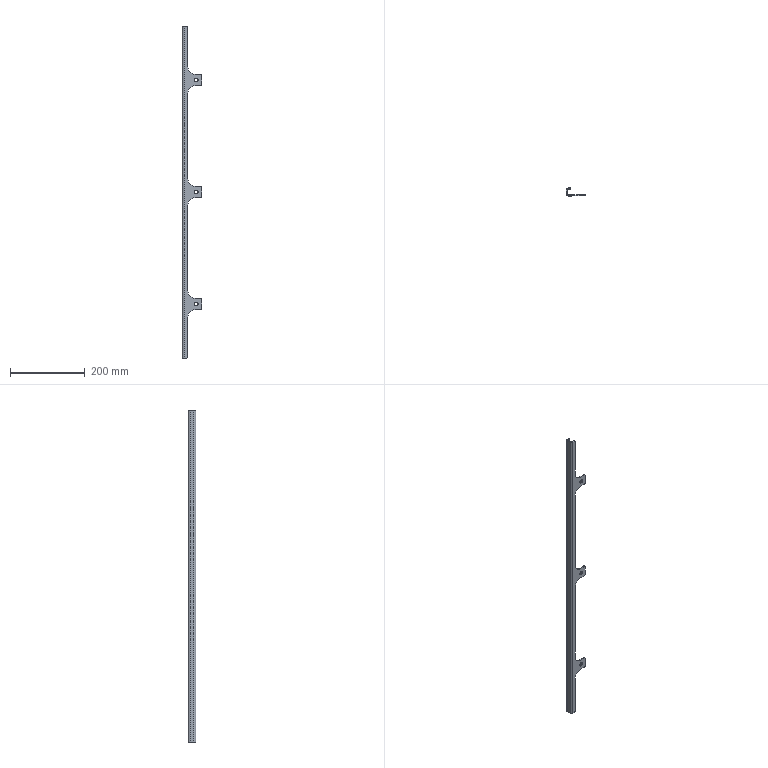Part | STEP file | 750078181 | 1 solid | 48 faces | box 52 x 20 x 889 mm | volume 95106 mm3 | cylinder 26 | plane 22 | commonest cylinder face diameters 6 x10 10.5 x6 40 x6 5 x2 10 x2
STEP:
#1=CARTESIAN_POINT('',(37.,2.5,5.25));
#2=VERTEX_POINT('',#1);
#3=CARTESIAN_POINT('',(37.,2.5,-5.25));
#4=VERTEX_POINT('',#3);
#5=CARTESIAN_POINT('',(37.,2.5,0.));
#6=DIRECTION('',(0.,-1.,0.));
#7=DIRECTION('',(0.,0.,-1.));
#8=AXIS2_PLACEMENT_3D('',#5,#6,#7);
#9=CIRCLE('',#8,5.25);
#10=EDGE_CURVE('',#2,#4,#9,.T.);
#11=ORIENTED_EDGE('',*,*,#10,.F.);
#12=CARTESIAN_POINT('',(37.,0.,5.25));
#13=VERTEX_POINT('',#12);
#14=CARTESIAN_POINT('',(37.,890.744,5.25));
#15=DIRECTION('',(0.,-1.,0.));
#16=VECTOR('',#15,1000.);
#17=LINE('',#14,#16);
#18=EDGE_CURVE('',#2,#13,#17,.T.);
#19=ORIENTED_EDGE('',*,*,#18,.T.);
#20=CARTESIAN_POINT('',(37.,0.,-5.25));
#21=VERTEX_POINT('',#20);
#22=CARTESIAN_POINT('',(37.,0.,0.));
#23=DIRECTION('',(0.,1.,0.));
#24=DIRECTION('',(0.,0.,-1.));
#25=AXIS2_PLACEMENT_3D('',#22,#23,#24);
#26=CIRCLE('',#25,5.25);
#27=EDGE_CURVE('',#21,#13,#26,.T.);
#28=ORIENTED_EDGE('',*,*,#27,.F.);
#29=CARTESIAN_POINT('',(37.,890.744,-5.25));
#30=DIRECTION('',(0.,-1.,0.));
#31=VECTOR('',#30,1000.);
#32=LINE('',#29,#31);
#33=EDGE_CURVE('',#4,#21,#32,.T.);
#34=ORIENTED_EDGE('',*,*,#33,.F.);
#35=EDGE_LOOP('',(#11,#19,#28,#34));
#36=FACE_OUTER_BOUND('',#35,.T.);
#37=CARTESIAN_POINT('',(37.,890.744,0.));
#38=DIRECTION('',(0.,-1.,0.));
#39=DIRECTION('',(0.,0.,-1.));
#40=AXIS2_PLACEMENT_3D('',#37,#38,#39);
#41=CYLINDRICAL_SURFACE('',#40,5.25);
#42=ADVANCED_FACE('',(#36),#41,.F.);
#43=CARTESIAN_POINT('',(37.,2.5,-294.75));
#44=VERTEX_POINT('',#43);
#45=CARTESIAN_POINT('',(37.,2.5,-305.25));
#46=VERTEX_POINT('',#45);
#47=CARTESIAN_POINT('',(37.,2.5,-300.));
#48=DIRECTION('',(0.,-1.,0.));
#49=DIRECTION('',(0.,0.,-1.));
#50=AXIS2_PLACEMENT_3D('',#47,#48,#49);
#51=CIRCLE('',#50,5.25);
#52=EDGE_CURVE('',#44,#46,#51,.T.);
#53=ORIENTED_EDGE('',*,*,#52,.F.);
#54=CARTESIAN_POINT('',(37.,0.,-294.75));
#55=VERTEX_POINT('',#54);
#56=CARTESIAN_POINT('',(37.,890.744,-294.75));
#57=DIRECTION('',(0.,-1.,0.));
#58=VECTOR('',#57,1000.);
#59=LINE('',#56,#58);
#60=EDGE_CURVE('',#44,#55,#59,.T.);
#61=ORIENTED_EDGE('',*,*,#60,.T.);
#62=CARTESIAN_POINT('',(37.,0.,-305.25));
#63=VERTEX_POINT('',#62);
#64=CARTESIAN_POINT('',(37.,0.,-300.));
#65=DIRECTION('',(0.,1.,0.));
#66=DIRECTION('',(0.,0.,-1.));
#67=AXIS2_PLACEMENT_3D('',#64,#65,#66);
#68=CIRCLE('',#67,5.25);
#69=EDGE_CURVE('',#63,#55,#68,.T.);
#70=ORIENTED_EDGE('',*,*,#69,.F.);
#71=CARTESIAN_POINT('',(37.,890.744,-305.25));
#72=DIRECTION('',(0.,-1.,0.));
#73=VECTOR('',#72,1000.);
#74=LINE('',#71,#73);
#75=EDGE_CURVE('',#46,#63,#74,.T.);
#76=ORIENTED_EDGE('',*,*,#75,.F.);
#77=EDGE_LOOP('',(#53,#61,#70,#76));
#78=FACE_OUTER_BOUND('',#77,.T.);
#79=CARTESIAN_POINT('',(37.,890.744,-300.));
#80=DIRECTION('',(0.,-1.,0.));
#81=DIRECTION('',(0.,0.,-1.));
#82=AXIS2_PLACEMENT_3D('',#79,#80,#81);
#83=CYLINDRICAL_SURFACE('',#82,5.25);
#84=ADVANCED_FACE('',(#78),#83,.F.);
#85=CARTESIAN_POINT('',(37.,2.5,305.25));
#86=VERTEX_POINT('',#85);
#87=CARTESIAN_POINT('',(37.,2.5,294.75));
#88=VERTEX_POINT('',#87);
#89=CARTESIAN_POINT('',(37.,2.5,300.));
#90=DIRECTION('',(0.,-1.,0.));
#91=DIRECTION('',(0.,0.,-1.));
#92=AXIS2_PLACEMENT_3D('',#89,#90,#91);
#93=CIRCLE('',#92,5.25);
#94=EDGE_CURVE('',#86,#88,#93,.T.);
#95=ORIENTED_EDGE('',*,*,#94,.F.);
#96=CARTESIAN_POINT('',(37.,0.,305.25));
#97=VERTEX_POINT('',#96);
#98=CARTESIAN_POINT('',(37.,890.744,305.25));
#99=DIRECTION('',(0.,-1.,0.));
#100=VECTOR('',#99,1000.);
#101=LINE('',#98,#100);
#102=EDGE_CURVE('',#86,#97,#101,.T.);
#103=ORIENTED_EDGE('',*,*,#102,.T.);
#104=CARTESIAN_POINT('',(37.,0.,294.75));
#105=VERTEX_POINT('',#104);
#106=CARTESIAN_POINT('',(37.,0.,300.));
#107=DIRECTION('',(0.,1.,0.));
#108=DIRECTION('',(0.,0.,-1.));
#109=AXIS2_PLACEMENT_3D('',#106,#107,#108);
#110=CIRCLE('',#109,5.25);
#111=EDGE_CURVE('',#105,#97,#110,.T.);
#112=ORIENTED_EDGE('',*,*,#111,.F.);
#113=CARTESIAN_POINT('',(37.,890.744,294.75));
#114=DIRECTION('',(0.,-1.,0.));
#115=VECTOR('',#114,1000.);
#116=LINE('',#113,#115);
#117=EDGE_CURVE('',#88,#105,#116,.T.);
#118=ORIENTED_EDGE('',*,*,#117,.F.);
#119=EDGE_LOOP('',(#95,#103,#112,#118));
#120=FACE_OUTER_BOUND('',#119,.T.);
#121=CARTESIAN_POINT('',(37.,890.744,300.));
#122=DIRECTION('',(0.,-1.,0.));
#123=DIRECTION('',(0.,0.,-1.));
#124=AXIS2_PLACEMENT_3D('',#121,#122,#123);
#125=CYLINDRICAL_SURFACE('',#124,5.25);
#126=ADVANCED_FACE('',(#120),#125,.F.);
#127=CARTESIAN_POINT('',(35.,0.,-15.));
#128=VERTEX_POINT('',#127);
#129=CARTESIAN_POINT('',(49.,0.,-15.));
#130=VERTEX_POINT('',#129);
#131=CARTESIAN_POINT('',(52.,0.,-15.));
#132=DIRECTION('',(1.,0.,0.));
#133=VECTOR('',#132,1000.);
#134=LINE('',#131,#133);
#135=EDGE_CURVE('',#128,#130,#134,.T.);
#136=ORIENTED_EDGE('',*,*,#135,.T.);
#137=CARTESIAN_POINT('',(52.,0.,-12.));
#138=VERTEX_POINT('',#137);
#139=CARTESIAN_POINT('',(49.,0.,-12.));
#140=DIRECTION('',(0.,-1.,0.));
#141=DIRECTION('',(0.,0.,-1.));
#142=AXIS2_PLACEMENT_3D('',#139,#140,#141);
#143=CIRCLE('',#142,3.);
#144=EDGE_CURVE('',#130,#138,#143,.T.);
#145=ORIENTED_EDGE('',*,*,#144,.T.);
#146=CARTESIAN_POINT('',(52.,0.,12.));
#147=VERTEX_POINT('',#146);
#148=CARTESIAN_POINT('',(52.,0.,444.5));
#149=DIRECTION('',(0.,0.,1.));
#150=VECTOR('',#149,1000.);
#151=LINE('',#148,#150);
#152=EDGE_CURVE('',#138,#147,#151,.T.);
#153=ORIENTED_EDGE('',*,*,#152,.T.);
#154=CARTESIAN_POINT('',(49.,0.,15.));
#155=VERTEX_POINT('',#154);
#156=CARTESIAN_POINT('',(49.,0.,12.));
#157=DIRECTION('',(0.,-1.,0.));
#158=DIRECTION('',(0.,0.,-1.));
#159=AXIS2_PLACEMENT_3D('',#156,#157,#158);
#160=CIRCLE('',#159,3.);
#161=EDGE_CURVE('',#147,#155,#160,.T.);
#162=ORIENTED_EDGE('',*,*,#161,.T.);
#163=CARTESIAN_POINT('',(35.,0.,15.));
#164=VERTEX_POINT('',#163);
#165=CARTESIAN_POINT('',(52.,0.,15.));
#166=DIRECTION('',(-1.,0.,0.));
#167=VECTOR('',#166,1000.);
#168=LINE('',#165,#167);
#169=EDGE_CURVE('',#155,#164,#168,.T.);
#170=ORIENTED_EDGE('',*,*,#169,.T.);
#171=CARTESIAN_POINT('',(15.,0.,35.));
#172=VERTEX_POINT('',#171);
#173=CARTESIAN_POINT('',(35.,0.,35.));
#174=DIRECTION('',(0.,1.,0.));
#175=DIRECTION('',(0.,0.,-1.));
#176=AXIS2_PLACEMENT_3D('',#173,#174,#175);
#177=CIRCLE('',#176,20.);
#178=EDGE_CURVE('',#164,#172,#177,.T.);
#179=ORIENTED_EDGE('',*,*,#178,.T.);
#180=CARTESIAN_POINT('',(15.,0.,265.));
#181=VERTEX_POINT('',#180);
#182=CARTESIAN_POINT('',(15.,0.,444.5));
#183=DIRECTION('',(0.,0.,1.));
#184=VECTOR('',#183,1000.);
#185=LINE('',#182,#184);
#186=EDGE_CURVE('',#172,#181,#185,.T.);
#187=ORIENTED_EDGE('',*,*,#186,.T.);
#188=CARTESIAN_POINT('',(35.,0.,285.));
#189=VERTEX_POINT('',#188);
#190=CARTESIAN_POINT('',(35.,0.,265.));
#191=DIRECTION('',(0.,1.,0.));
#192=DIRECTION('',(0.,0.,-1.));
#193=AXIS2_PLACEMENT_3D('',#190,#191,#192);
#194=CIRCLE('',#193,20.);
#195=EDGE_CURVE('',#181,#189,#194,.T.);
#196=ORIENTED_EDGE('',*,*,#195,.T.);
#197=CARTESIAN_POINT('',(49.,0.,285.));
#198=VERTEX_POINT('',#197);
#199=CARTESIAN_POINT('',(52.,0.,285.));
#200=DIRECTION('',(1.,0.,0.));
#201=VECTOR('',#200,1000.);
#202=LINE('',#199,#201);
#203=EDGE_CURVE('',#189,#198,#202,.T.);
#204=ORIENTED_EDGE('',*,*,#203,.T.);
#205=CARTESIAN_POINT('',(52.,0.,288.));
#206=VERTEX_POINT('',#205);
#207=CARTESIAN_POINT('',(49.,0.,288.));
#208=DIRECTION('',(0.,-1.,0.));
#209=DIRECTION('',(0.,0.,-1.));
#210=AXIS2_PLACEMENT_3D('',#207,#208,#209);
#211=CIRCLE('',#210,3.);
#212=EDGE_CURVE('',#198,#206,#211,.T.);
#213=ORIENTED_EDGE('',*,*,#212,.T.);
#214=CARTESIAN_POINT('',(52.,0.,312.));
#215=VERTEX_POINT('',#214);
#216=CARTESIAN_POINT('',(52.,0.,444.5));
#217=DIRECTION('',(0.,0.,1.));
#218=VECTOR('',#217,1000.);
#219=LINE('',#216,#218);
#220=EDGE_CURVE('',#206,#215,#219,.T.);
#221=ORIENTED_EDGE('',*,*,#220,.T.);
#222=CARTESIAN_POINT('',(49.,0.,315.));
#223=VERTEX_POINT('',#222);
#224=CARTESIAN_POINT('',(49.,0.,312.));
#225=DIRECTION('',(0.,-1.,0.));
#226=DIRECTION('',(0.,0.,-1.));
#227=AXIS2_PLACEMENT_3D('',#224,#225,#226);
#228=CIRCLE('',#227,3.);
#229=EDGE_CURVE('',#215,#223,#228,.T.);
#230=ORIENTED_EDGE('',*,*,#229,.T.);
#231=CARTESIAN_POINT('',(35.,0.,315.));
#232=VERTEX_POINT('',#231);
#233=CARTESIAN_POINT('',(52.,0.,315.));
#234=DIRECTION('',(-1.,0.,0.));
#235=VECTOR('',#234,1000.);
#236=LINE('',#233,#235);
#237=EDGE_CURVE('',#223,#232,#236,.T.);
#238=ORIENTED_EDGE('',*,*,#237,.T.);
#239=CARTESIAN_POINT('',(15.,0.,335.));
#240=VERTEX_POINT('',#239);
#241=CARTESIAN_POINT('',(35.,0.,335.));
#242=DIRECTION('',(0.,1.,0.));
#243=DIRECTION('',(0.,0.,-1.));
#244=AXIS2_PLACEMENT_3D('',#241,#242,#243);
#245=CIRCLE('',#244,20.);
#246=EDGE_CURVE('',#232,#240,#245,.T.);
#247=ORIENTED_EDGE('',*,*,#246,.T.);
#248=CARTESIAN_POINT('',(15.,0.,441.5));
#249=VERTEX_POINT('',#248);
#250=CARTESIAN_POINT('',(15.,0.,444.5));
#251=DIRECTION('',(0.,0.,1.));
#252=VECTOR('',#251,1000.);
#253=LINE('',#250,#252);
#254=EDGE_CURVE('',#240,#249,#253,.T.);
#255=ORIENTED_EDGE('',*,*,#254,.T.);
#256=CARTESIAN_POINT('',(12.,0.,444.5));
#257=VERTEX_POINT('',#256);
#258=CARTESIAN_POINT('',(12.,0.,441.5));
#259=DIRECTION('',(0.,-1.,0.));
#260=DIRECTION('',(0.,0.,1.));
#261=AXIS2_PLACEMENT_3D('',#258,#259,#260);
#262=CIRCLE('',#261,3.);
#263=EDGE_CURVE('',#249,#257,#262,.T.);
#264=ORIENTED_EDGE('',*,*,#263,.T.);
#265=CARTESIAN_POINT('',(5.,0.,444.5));
#266=VERTEX_POINT('',#265);
#267=CARTESIAN_POINT('',(52.,0.,444.5));
#268=DIRECTION('',(-1.,0.,0.));
#269=VECTOR('',#268,1000.);
#270=LINE('',#267,#269);
#271=EDGE_CURVE('',#257,#266,#270,.T.);
#272=ORIENTED_EDGE('',*,*,#271,.T.);
#273=CARTESIAN_POINT('',(5.,0.,-444.5));
#274=VERTEX_POINT('',#273);
#275=CARTESIAN_POINT('',(5.,0.,444.5));
#276=DIRECTION('',(0.,0.,-1.));
#277=VECTOR('',#276,1000.);
#278=LINE('',#275,#277);
#279=EDGE_CURVE('',#266,#274,#278,.T.);
#280=ORIENTED_EDGE('',*,*,#279,.T.);
#281=CARTESIAN_POINT('',(12.,0.,-444.5));
#282=VERTEX_POINT('',#281);
#283=CARTESIAN_POINT('',(52.,0.,-444.5));
#284=DIRECTION('',(1.,0.,0.));
#285=VECTOR('',#284,1000.);
#286=LINE('',#283,#285);
#287=EDGE_CURVE('',#274,#282,#286,.T.);
#288=ORIENTED_EDGE('',*,*,#287,.T.);
#289=CARTESIAN_POINT('',(15.,0.,-441.5));
#290=VERTEX_POINT('',#289);
#291=CARTESIAN_POINT('',(12.,0.,-441.5));
#292=DIRECTION('',(0.,-1.,0.));
#293=DIRECTION('',(0.,0.,-1.));
#294=AXIS2_PLACEMENT_3D('',#291,#292,#293);
#295=CIRCLE('',#294,3.);
#296=EDGE_CURVE('',#282,#290,#295,.T.);
#297=ORIENTED_EDGE('',*,*,#296,.T.);
#298=CARTESIAN_POINT('',(15.,0.,-335.));
#299=VERTEX_POINT('',#298);
#300=CARTESIAN_POINT('',(15.,0.,444.5));
#301=DIRECTION('',(0.,0.,1.));
#302=VECTOR('',#301,1000.);
#303=LINE('',#300,#302);
#304=EDGE_CURVE('',#290,#299,#303,.T.);
#305=ORIENTED_EDGE('',*,*,#304,.T.);
#306=CARTESIAN_POINT('',(35.,0.,-315.));
#307=VERTEX_POINT('',#306);
#308=CARTESIAN_POINT('',(35.,0.,-335.));
#309=DIRECTION('',(0.,1.,0.));
#310=DIRECTION('',(0.,0.,-1.));
#311=AXIS2_PLACEMENT_3D('',#308,#309,#310);
#312=CIRCLE('',#311,20.);
#313=EDGE_CURVE('',#299,#307,#312,.T.);
#314=ORIENTED_EDGE('',*,*,#313,.T.);
#315=CARTESIAN_POINT('',(49.,0.,-315.));
#316=VERTEX_POINT('',#315);
#317=CARTESIAN_POINT('',(52.,0.,-315.));
#318=DIRECTION('',(1.,0.,0.));
#319=VECTOR('',#318,1000.);
#320=LINE('',#317,#319);
#321=EDGE_CURVE('',#307,#316,#320,.T.);
#322=ORIENTED_EDGE('',*,*,#321,.T.);
#323=CARTESIAN_POINT('',(52.,0.,-312.));
#324=VERTEX_POINT('',#323);
#325=CARTESIAN_POINT('',(49.,0.,-312.));
#326=DIRECTION('',(0.,-1.,0.));
#327=DIRECTION('',(0.,0.,-1.));
#328=AXIS2_PLACEMENT_3D('',#325,#326,#327);
#329=CIRCLE('',#328,3.);
#330=EDGE_CURVE('',#316,#324,#329,.T.);
#331=ORIENTED_EDGE('',*,*,#330,.T.);
#332=CARTESIAN_POINT('',(52.,0.,-288.));
#333=VERTEX_POINT('',#332);
#334=CARTESIAN_POINT('',(52.,0.,444.5));
#335=DIRECTION('',(0.,0.,1.));
#336=VECTOR('',#335,1000.);
#337=LINE('',#334,#336);
#338=EDGE_CURVE('',#324,#333,#337,.T.);
#339=ORIENTED_EDGE('',*,*,#338,.T.);
#340=CARTESIAN_POINT('',(49.,0.,-285.));
#341=VERTEX_POINT('',#340);
#342=CARTESIAN_POINT('',(49.,0.,-288.));
#343=DIRECTION('',(0.,-1.,0.));
#344=DIRECTION('',(0.,0.,-1.));
#345=AXIS2_PLACEMENT_3D('',#342,#343,#344);
#346=CIRCLE('',#345,3.);
#347=EDGE_CURVE('',#333,#341,#346,.T.);
#348=ORIENTED_EDGE('',*,*,#347,.T.);
#349=CARTESIAN_POINT('',(35.,0.,-285.));
#350=VERTEX_POINT('',#349);
#351=CARTESIAN_POINT('',(52.,0.,-285.));
#352=DIRECTION('',(-1.,0.,0.));
#353=VECTOR('',#352,1000.);
#354=LINE('',#351,#353);
#355=EDGE_CURVE('',#341,#350,#354,.T.);
#356=ORIENTED_EDGE('',*,*,#355,.T.);
#357=CARTESIAN_POINT('',(15.,0.,-265.));
#358=VERTEX_POINT('',#357);
#359=CARTESIAN_POINT('',(35.,0.,-265.));
#360=DIRECTION('',(0.,1.,0.));
#361=DIRECTION('',(0.,0.,-1.));
#362=AXIS2_PLACEMENT_3D('',#359,#360,#361);
#363=CIRCLE('',#362,20.);
#364=EDGE_CURVE('',#350,#358,#363,.T.);
#365=ORIENTED_EDGE('',*,*,#364,.T.);
#366=CARTESIAN_POINT('',(15.,0.,-35.));
#367=VERTEX_POINT('',#366);
#368=CARTESIAN_POINT('',(15.,0.,444.5));
#369=DIRECTION('',(0.,0.,1.));
#370=VECTOR('',#369,1000.);
#371=LINE('',#368,#370);
#372=EDGE_CURVE('',#358,#367,#371,.T.);
#373=ORIENTED_EDGE('',*,*,#372,.T.);
#374=CARTESIAN_POINT('',(35.,0.,-35.));
#375=DIRECTION('',(0.,1.,0.));
#376=DIRECTION('',(0.,0.,-1.));
#377=AXIS2_PLACEMENT_3D('',#374,#375,#376);
#378=CIRCLE('',#377,20.);
#379=EDGE_CURVE('',#367,#128,#378,.T.);
#380=ORIENTED_EDGE('',*,*,#379,.T.);
#381=EDGE_LOOP('',(#136,#145,#153,#162,#170,#179,#187,#196,#204,#213,#221,#230,#238,#247,#255,#264,#272,#280,#288,#297,#305,#314,#322,#331,#339,#348,#356,#365,#373,#380));
#382=FACE_OUTER_BOUND('',#381,.T.);
#383=ORIENTED_EDGE('',*,*,#27,.T.);
#384=CARTESIAN_POINT('',(37.,0.,0.));
#385=DIRECTION('',(0.,1.,0.));
#386=DIRECTION('',(0.,0.,-1.));
#387=AXIS2_PLACEMENT_3D('',#384,#385,#386);
#388=CIRCLE('',#387,5.25);
#389=EDGE_CURVE('',#13,#21,#388,.T.);
#390=ORIENTED_EDGE('',*,*,#389,.T.);
#391=EDGE_LOOP('',(#383,#390));
#392=FACE_BOUND('',#391,.T.);
#393=ORIENTED_EDGE('',*,*,#69,.T.);
#394=CARTESIAN_POINT('',(37.,0.,-300.));
#395=DIRECTION('',(0.,1.,0.));
#396=DIRECTION('',(0.,0.,-1.));
#397=AXIS2_PLACEMENT_3D('',#394,#395,#396);
#398=CIRCLE('',#397,5.25);
#399=EDGE_CURVE('',#55,#63,#398,.T.);
#400=ORIENTED_EDGE('',*,*,#399,.T.);
#401=EDGE_LOOP('',(#393,#400));
#402=FACE_BOUND('',#401,.T.);
#403=ORIENTED_EDGE('',*,*,#111,.T.);
#404=CARTESIAN_POINT('',(37.,0.,300.));
#405=DIRECTION('',(0.,1.,0.));
#406=DIRECTION('',(0.,0.,-1.));
#407=AXIS2_PLACEMENT_3D('',#404,#405,#406);
#408=CIRCLE('',#407,5.25);
#409=EDGE_CURVE('',#97,#105,#408,.T.);
#410=ORIENTED_EDGE('',*,*,#409,.T.);
#411=EDGE_LOOP('',(#403,#410));
#412=FACE_BOUND('',#411,.T.);
#413=CARTESIAN_POINT('',(52.,0.,444.5));
#414=DIRECTION('',(0.,-1.,0.));
#415=DIRECTION('',(0.,0.,-1.));
#416=AXIS2_PLACEMENT_3D('',#413,#414,#415);
#417=PLANE('',#416);
#418=ADVANCED_FACE('',(#382,#392,#402,#412),#417,.T.);
#419=ORIENTED_EDGE('',*,*,#144,.F.);
#420=CARTESIAN_POINT('',(49.,2.5,-15.));
#421=VERTEX_POINT('',#420);
#422=CARTESIAN_POINT('',(49.,5.,-15.));
#423=DIRECTION('',(0.,1.,0.));
#424=VECTOR('',#423,1000.);
#425=LINE('',#422,#424);
#426=EDGE_CURVE('',#130,#421,#425,.T.);
#427=ORIENTED_EDGE('',*,*,#426,.T.);
#428=CARTESIAN_POINT('',(52.,2.5,-12.));
#429=VERTEX_POINT('',#428);
#430=CARTESIAN_POINT('',(49.,2.5,-12.));
#431=DIRECTION('',(0.,-1.,0.));
#432=DIRECTION('',(0.,0.,-1.));
#433=AXIS2_PLACEMENT_3D('',#430,#431,#432);
#434=CIRCLE('',#433,3.);
#435=EDGE_CURVE('',#421,#429,#434,.T.);
#436=ORIENTED_EDGE('',*,*,#435,.T.);
#437=CARTESIAN_POINT('',(52.,5.,-12.));
#438=DIRECTION('',(0.,-1.,0.));
#439=VECTOR('',#438,1000.);
#440=LINE('',#437,#439);
#441=EDGE_CURVE('',#429,#138,#440,.T.);
#442=ORIENTED_EDGE('',*,*,#441,.T.);
#443=EDGE_LOOP('',(#419,#427,#436,#442));
#444=FACE_OUTER_BOUND('',#443,.T.);
#445=CARTESIAN_POINT('',(49.,5.,-12.));
#446=DIRECTION('',(0.,-1.,0.));
#447=DIRECTION('',(0.,0.,-1.));
#448=AXIS2_PLACEMENT_3D('',#445,#446,#447);
#449=CYLINDRICAL_SURFACE('',#448,3.);
#450=ADVANCED_FACE('',(#444),#449,.T.);
#451=ORIENTED_EDGE('',*,*,#426,.F.);
#452=ORIENTED_EDGE('',*,*,#135,.F.);
#453=CARTESIAN_POINT('',(35.,2.5,-15.));
#454=VERTEX_POINT('',#453);
#455=CARTESIAN_POINT('',(35.,5.,-15.));
#456=DIRECTION('',(0.,-1.,0.));
#457=VECTOR('',#456,1000.);
#458=LINE('',#455,#457);
#459=EDGE_CURVE('',#454,#128,#458,.T.);
#460=ORIENTED_EDGE('',*,*,#459,.F.);
#461=CARTESIAN_POINT('',(53.,2.5,-15.));
#462=DIRECTION('',(-1.,0.,0.));
#463=VECTOR('',#462,1000.);
#464=LINE('',#461,#463);
#465=EDGE_CURVE('',#421,#454,#464,.T.);
#466=ORIENTED_EDGE('',*,*,#465,.F.);
#467=EDGE_LOOP('',(#451,#452,#460,#466));
#468=FACE_OUTER_BOUND('',#467,.T.);
#469=CARTESIAN_POINT('',(53.,5.,-15.));
#470=DIRECTION('',(0.,0.,1.));
#471=DIRECTION('',(1.,0.,0.));
#472=AXIS2_PLACEMENT_3D('',#469,#470,#471);
#473=PLANE('',#472);
#474=ADVANCED_FACE('',(#468),#473,.F.);
#475=CARTESIAN_POINT('',(15.,2.5,-35.));
#476=VERTEX_POINT('',#475);
#477=CARTESIAN_POINT('',(15.,5.,-35.));
#478=DIRECTION('',(0.,-1.,0.));
#479=VECTOR('',#478,1000.);
#480=LINE('',#477,#479);
#481=EDGE_CURVE('',#476,#367,#480,.T.);
#482=ORIENTED_EDGE('',*,*,#481,.F.);
#483=CARTESIAN_POINT('',(35.,2.5,-35.));
#484=DIRECTION('',(0.,-1.,0.));
#485=DIRECTION('',(0.,0.,-1.));
#486=AXIS2_PLACEMENT_3D('',#483,#484,#485);
#487=CIRCLE('',#486,20.);
#488=EDGE_CURVE('',#454,#476,#487,.T.);
#489=ORIENTED_EDGE('',*,*,#488,.F.);
#490=ORIENTED_EDGE('',*,*,#459,.T.);
#491=ORIENTED_EDGE('',*,*,#379,.F.);
#492=EDGE_LOOP('',(#482,#489,#490,#491));
#493=FACE_OUTER_BOUND('',#492,.T.);
#494=CARTESIAN_POINT('',(35.,5.,-35.));
#495=DIRECTION('',(0.,-1.,0.));
#496=DIRECTION('',(0.,0.,-1.));
#497=AXIS2_PLACEMENT_3D('',#494,#495,#496);
#498=CYLINDRICAL_SURFACE('',#497,20.);
#499=ADVANCED_FACE('',(#493),#498,.F.);
#500=ORIENTED_EDGE('',*,*,#481,.T.);
#501=ORIENTED_EDGE('',*,*,#372,.F.);
#502=CARTESIAN_POINT('',(15.,2.5,-265.));
#503=VERTEX_POINT('',#502);
#504=CARTESIAN_POINT('',(15.,5.,-265.));
#505=DIRECTION('',(0.,-1.,0.));
#506=VECTOR('',#505,1000.);
#507=LINE('',#504,#506);
#508=EDGE_CURVE('',#503,#358,#507,.T.);
#509=ORIENTED_EDGE('',*,*,#508,.F.);
#510=CARTESIAN_POINT('',(15.,2.5,-15.));
#511=DIRECTION('',(0.,0.,-1.));
#512=VECTOR('',#511,1000.);
#513=LINE('',#510,#512);
#514=EDGE_CURVE('',#476,#503,#513,.T.);
#515=ORIENTED_EDGE('',*,*,#514,.F.);
#516=EDGE_LOOP('',(#500,#501,#509,#515));
#517=FACE_OUTER_BOUND('',#516,.T.);
#518=CARTESIAN_POINT('',(15.,5.,-15.));
#519=DIRECTION('',(-1.,0.,0.));
#520=DIRECTION('',(0.,0.,1.));
#521=AXIS2_PLACEMENT_3D('',#518,#519,#520);
#522=PLANE('',#521);
#523=ADVANCED_FACE('',(#517),#522,.F.);
#524=CARTESIAN_POINT('',(35.,2.5,-285.));
#525=VERTEX_POINT('',#524);
#526=CARTESIAN_POINT('',(35.,5.,-285.));
#527=DIRECTION('',(0.,-1.,0.));
#528=VECTOR('',#527,1000.);
#529=LINE('',#526,#528);
#530=EDGE_CURVE('',#525,#350,#529,.T.);
#531=ORIENTED_EDGE('',*,*,#530,.F.);
#532=CARTESIAN_POINT('',(35.,2.5,-265.));
#533=DIRECTION('',(0.,-1.,0.));
#534=DIRECTION('',(0.,0.,-1.));
#535=AXIS2_PLACEMENT_3D('',#532,#533,#534);
#536=CIRCLE('',#535,20.);
#537=EDGE_CURVE('',#503,#525,#536,.T.);
#538=ORIENTED_EDGE('',*,*,#537,.F.);
#539=ORIENTED_EDGE('',*,*,#508,.T.);
#540=ORIENTED_EDGE('',*,*,#364,.F.);
#541=EDGE_LOOP('',(#531,#538,#539,#540));
#542=FACE_OUTER_BOUND('',#541,.T.);
#543=CARTESIAN_POINT('',(35.,5.,-265.));
#544=DIRECTION('',(0.,-1.,0.));
#545=DIRECTION('',(0.,0.,-1.));
#546=AXIS2_PLACEMENT_3D('',#543,#544,#545);
#547=CYLINDRICAL_SURFACE('',#546,20.);
#548=ADVANCED_FACE('',(#542),#547,.F.);
#549=CARTESIAN_POINT('',(49.,2.5,-285.));
#550=VERTEX_POINT('',#549);
#551=CARTESIAN_POINT('',(49.,5.,-285.));
#552=DIRECTION('',(0.,-1.,0.));
#553=VECTOR('',#552,1000.);
#554=LINE('',#551,#553);
#555=EDGE_CURVE('',#550,#341,#554,.T.);
#556=ORIENTED_EDGE('',*,*,#555,.F.);
#557=CARTESIAN_POINT('',(15.,2.5,-285.));
#558=DIRECTION('',(1.,0.,0.));
#559=VECTOR('',#558,1000.);
#560=LINE('',#557,#559);
#561=EDGE_CURVE('',#525,#550,#560,.T.);
#562=ORIENTED_EDGE('',*,*,#561,.F.);
#563=ORIENTED_EDGE('',*,*,#530,.T.);
#564=ORIENTED_EDGE('',*,*,#355,.F.);
#565=EDGE_LOOP('',(#556,#562,#563,#564));
#566=FACE_OUTER_BOUND('',#565,.T.);
#567=CARTESIAN_POINT('',(15.,5.,-285.));
#568=DIRECTION('',(0.,0.,-1.));
#569=DIRECTION('',(-1.,0.,0.));
#570=AXIS2_PLACEMENT_3D('',#567,#568,#569);
#571=PLANE('',#570);
#572=ADVANCED_FACE('',(#566),#571,.F.);
#573=ORIENTED_EDGE('',*,*,#347,.F.);
#574=CARTESIAN_POINT('',(52.,2.5,-288.));
#575=VERTEX_POINT('',#574);
#576=CARTESIAN_POINT('',(52.,0.,-288.));
#577=DIRECTION('',(0.,1.,0.));
#578=VECTOR('',#577,1000.);
#579=LINE('',#576,#578);
#580=EDGE_CURVE('',#333,#575,#579,.T.);
#581=ORIENTED_EDGE('',*,*,#580,.T.);
#582=CARTESIAN_POINT('',(49.,2.5,-288.));
#583=DIRECTION('',(0.,-1.,0.));
#584=DIRECTION('',(0.,0.,-1.));
#585=AXIS2_PLACEMENT_3D('',#582,#583,#584);
#586=CIRCLE('',#585,3.);
#587=EDGE_CURVE('',#575,#550,#586,.T.);
#588=ORIENTED_EDGE('',*,*,#587,.T.);
#589=ORIENTED_EDGE('',*,*,#555,.T.);
#590=EDGE_LOOP('',(#573,#581,#588,#589));
#591=FACE_OUTER_BOUND('',#590,.T.);
#592=CARTESIAN_POINT('',(49.,0.,-288.));
#593=DIRECTION('',(0.,-1.,0.));
#594=DIRECTION('',(0.,0.,-1.));
#595=AXIS2_PLACEMENT_3D('',#592,#593,#594);
#596=CYLINDRICAL_SURFACE('',#595,3.);
#597=ADVANCED_FACE('',(#591),#596,.T.);
#598=ORIENTED_EDGE('',*,*,#580,.F.);
#599=ORIENTED_EDGE('',*,*,#338,.F.);
#600=CARTESIAN_POINT('',(52.,2.5,-312.));
#601=VERTEX_POINT('',#600);
#602=CARTESIAN_POINT('',(52.,0.,-312.));
#603=DIRECTION('',(0.,-1.,0.));
#604=VECTOR('',#603,1000.);
#605=LINE('',#602,#604);
#606=EDGE_CURVE('',#601,#324,#605,.T.);
#607=ORIENTED_EDGE('',*,*,#606,.F.);
#608=CARTESIAN_POINT('',(52.,2.5,444.5));
#609=DIRECTION('',(0.,0.,-1.));
#610=VECTOR('',#609,1000.);
#611=LINE('',#608,#610);
#612=EDGE_CURVE('',#575,#601,#611,.T.);
#613=ORIENTED_EDGE('',*,*,#612,.F.);
#614=EDGE_LOOP('',(#598,#599,#607,#613));
#615=FACE_OUTER_BOUND('',#614,.T.);
#616=CARTESIAN_POINT('',(52.,0.,444.5));
#617=DIRECTION('',(-1.,0.,0.));
#618=DIRECTION('',(0.,0.,1.));
#619=AXIS2_PLACEMENT_3D('',#616,#617,#618);
#620=PLANE('',#619);
#621=ADVANCED_FACE('',(#615),#620,.F.);
#622=ORIENTED_EDGE('',*,*,#330,.F.);
#623=CARTESIAN_POINT('',(49.,2.5,-315.));
#624=VERTEX_POINT('',#623);
#625=CARTESIAN_POINT('',(49.,5.,-315.));
#626=DIRECTION('',(0.,1.,0.));
#627=VECTOR('',#626,1000.);
#628=LINE('',#625,#627);
#629=EDGE_CURVE('',#316,#624,#628,.T.);
#630=ORIENTED_EDGE('',*,*,#629,.T.);
#631=CARTESIAN_POINT('',(49.,2.5,-312.));
#632=DIRECTION('',(0.,-1.,0.));
#633=DIRECTION('',(0.,0.,-1.));
#634=AXIS2_PLACEMENT_3D('',#631,#632,#633);
#635=CIRCLE('',#634,3.);
#636=EDGE_CURVE('',#624,#601,#635,.T.);
#637=ORIENTED_EDGE('',*,*,#636,.T.);
#638=ORIENTED_EDGE('',*,*,#606,.T.);
#639=EDGE_LOOP('',(#622,#630,#637,#638));
#640=FACE_OUTER_BOUND('',#639,.T.);
#641=CARTESIAN_POINT('',(49.,5.,-312.));
#642=DIRECTION('',(0.,-1.,0.));
#643=DIRECTION('',(0.,0.,-1.));
#644=AXIS2_PLACEMENT_3D('',#641,#642,#643);
#645=CYLINDRICAL_SURFACE('',#644,3.);
#646=ADVANCED_FACE('',(#640),#645,.T.);
#647=ORIENTED_EDGE('',*,*,#629,.F.);
#648=ORIENTED_EDGE('',*,*,#321,.F.);
#649=CARTESIAN_POINT('',(35.,2.5,-315.));
#650=VERTEX_POINT('',#649);
#651=CARTESIAN_POINT('',(35.,5.,-315.));
#652=DIRECTION('',(0.,-1.,0.));
#653=VECTOR('',#652,1000.);
#654=LINE('',#651,#653);
#655=EDGE_CURVE('',#650,#307,#654,.T.);
#656=ORIENTED_EDGE('',*,*,#655,.F.);
#657=CARTESIAN_POINT('',(53.,2.5,-315.));
#658=DIRECTION('',(-1.,0.,0.));
#659=VECTOR('',#658,1000.);
#660=LINE('',#657,#659);
#661=EDGE_CURVE('',#624,#650,#660,.T.);
#662=ORIENTED_EDGE('',*,*,#661,.F.);
#663=EDGE_LOOP('',(#647,#648,#656,#662));
#664=FACE_OUTER_BOUND('',#663,.T.);
#665=CARTESIAN_POINT('',(53.,5.,-315.));
#666=DIRECTION('',(0.,0.,1.));
#667=DIRECTION('',(1.,0.,0.));
#668=AXIS2_PLACEMENT_3D('',#665,#666,#667);
#669=PLANE('',#668);
#670=ADVANCED_FACE('',(#664),#669,.F.);
#671=CARTESIAN_POINT('',(15.,2.5,-335.));
#672=VERTEX_POINT('',#671);
#673=CARTESIAN_POINT('',(15.,5.,-335.));
#674=DIRECTION('',(0.,-1.,0.));
#675=VECTOR('',#674,1000.);
#676=LINE('',#673,#675);
#677=EDGE_CURVE('',#672,#299,#676,.T.);
#678=ORIENTED_EDGE('',*,*,#677,.F.);
#679=CARTESIAN_POINT('',(35.,2.5,-335.));
#680=DIRECTION('',(0.,-1.,0.));
#681=DIRECTION('',(0.,0.,-1.));
#682=AXIS2_PLACEMENT_3D('',#679,#680,#681);
#683=CIRCLE('',#682,20.);
#684=EDGE_CURVE('',#650,#672,#683,.T.);
#685=ORIENTED_EDGE('',*,*,#684,.F.);
#686=ORIENTED_EDGE('',*,*,#655,.T.);
#687=ORIENTED_EDGE('',*,*,#313,.F.);
#688=EDGE_LOOP('',(#678,#685,#686,#687));
#689=FACE_OUTER_BOUND('',#688,.T.);
#690=CARTESIAN_POINT('',(35.,5.,-335.));
#691=DIRECTION('',(0.,-1.,0.));
#692=DIRECTION('',(0.,0.,-1.));
#693=AXIS2_PLACEMENT_3D('',#690,#691,#692);
#694=CYLINDRICAL_SURFACE('',#693,20.);
#695=ADVANCED_FACE('',(#689),#694,.F.);
#696=CARTESIAN_POINT('',(15.,2.5,-441.5));
#697=VERTEX_POINT('',#696);
#698=CARTESIAN_POINT('',(15.,5.,-441.5));
#699=DIRECTION('',(0.,-1.,0.));
#700=VECTOR('',#699,1000.);
#701=LINE('',#698,#700);
#702=EDGE_CURVE('',#697,#290,#701,.T.);
#703=ORIENTED_EDGE('',*,*,#702,.F.);
#704=CARTESIAN_POINT('',(15.,2.5,-315.));
#705=DIRECTION('',(0.,0.,-1.));
#706=VECTOR('',#705,1000.);
#707=LINE('',#704,#706);
#708=EDGE_CURVE('',#672,#697,#707,.T.);
#709=ORIENTED_EDGE('',*,*,#708,.F.);
#710=ORIENTED_EDGE('',*,*,#677,.T.);
#711=ORIENTED_EDGE('',*,*,#304,.F.);
#712=EDGE_LOOP('',(#703,#709,#710,#711));
#713=FACE_OUTER_BOUND('',#712,.T.);
#714=CARTESIAN_POINT('',(15.,5.,-315.));
#715=DIRECTION('',(-1.,0.,0.));
#716=DIRECTION('',(0.,0.,1.));
#717=AXIS2_PLACEMENT_3D('',#714,#715,#716);
#718=PLANE('',#717);
#719=ADVANCED_FACE('',(#713),#718,.F.);
#720=ORIENTED_EDGE('',*,*,#296,.F.);
#721=CARTESIAN_POINT('',(12.,2.5,-444.5));
#722=VERTEX_POINT('',#721);
#723=CARTESIAN_POINT('',(12.,0.,-444.5));
#724=DIRECTION('',(0.,1.,0.));
#725=VECTOR('',#724,1000.);
#726=LINE('',#723,#725);
#727=EDGE_CURVE('',#282,#722,#726,.T.);
#728=ORIENTED_EDGE('',*,*,#727,.T.);
#729=CARTESIAN_POINT('',(12.,2.5,-441.5));
#730=DIRECTION('',(0.,-1.,0.));
#731=DIRECTION('',(0.,0.,-1.));
#732=AXIS2_PLACEMENT_3D('',#729,#730,#731);
#733=CIRCLE('',#732,3.);
#734=EDGE_CURVE('',#722,#697,#733,.T.);
#735=ORIENTED_EDGE('',*,*,#734,.T.);
#736=ORIENTED_EDGE('',*,*,#702,.T.);
#737=EDGE_LOOP('',(#720,#728,#735,#736));
#738=FACE_OUTER_BOUND('',#737,.T.);
#739=CARTESIAN_POINT('',(12.,0.,-441.5));
#740=DIRECTION('',(0.,-1.,0.));
#741=DIRECTION('',(0.,0.,-1.));
#742=AXIS2_PLACEMENT_3D('',#739,#740,#741);
#743=CYLINDRICAL_SURFACE('',#742,3.);
#744=ADVANCED_FACE('',(#738),#743,.T.);
#745=ORIENTED_EDGE('',*,*,#727,.F.);
#746=ORIENTED_EDGE('',*,*,#287,.F.);
#747=CARTESIAN_POINT('',(0.,5.,-444.5));
#748=VERTEX_POINT('',#747);
#749=CARTESIAN_POINT('',(5.,5.,-444.5));
#750=DIRECTION('',(0.,0.,1.));
#751=DIRECTION('',(-1.,0.,0.));
#752=AXIS2_PLACEMENT_3D('',#749,#750,#751);
#753=CIRCLE('',#752,5.);
#754=EDGE_CURVE('',#748,#274,#753,.T.);
#755=ORIENTED_EDGE('',*,*,#754,.F.);
#756=CARTESIAN_POINT('',(0.,15.,-444.5));
#757=VERTEX_POINT('',#756);
#758=CARTESIAN_POINT('',(0.,0.,-444.5));
#759=DIRECTION('',(0.,-1.,0.));
#760=VECTOR('',#759,1000.);
#761=LINE('',#758,#760);
#762=EDGE_CURVE('',#757,#748,#761,.T.);
#763=ORIENTED_EDGE('',*,*,#762,.F.);
#764=CARTESIAN_POINT('',(5.,20.,-444.5));
#765=VERTEX_POINT('',#764);
#766=CARTESIAN_POINT('',(5.,15.,-444.5));
#767=DIRECTION('',(0.,0.,1.));
#768=DIRECTION('',(-1.,0.,0.));
#769=AXIS2_PLACEMENT_3D('',#766,#767,#768);
#770=CIRCLE('',#769,5.);
#771=EDGE_CURVE('',#765,#757,#770,.T.);
#772=ORIENTED_EDGE('',*,*,#771,.F.);
#773=CARTESIAN_POINT('',(9.,20.,-444.5));
#774=VERTEX_POINT('',#773);
#775=CARTESIAN_POINT('',(52.,20.,-444.5));
#776=DIRECTION('',(-1.,0.,0.));
#777=VECTOR('',#776,1000.);
#778=LINE('',#775,#777);
#779=EDGE_CURVE('',#774,#765,#778,.T.);
#780=ORIENTED_EDGE('',*,*,#779,.F.);
#781=CARTESIAN_POINT('',(9.,17.5,-444.5));
#782=VERTEX_POINT('',#781);
#783=CARTESIAN_POINT('',(9.,0.,-444.5));
#784=DIRECTION('',(0.,1.,0.));
#785=VECTOR('',#784,1000.);
#786=LINE('',#783,#785);
#787=EDGE_CURVE('',#782,#774,#786,.T.);
#788=ORIENTED_EDGE('',*,*,#787,.F.);
#789=CARTESIAN_POINT('',(5.,17.5,-444.5));
#790=VERTEX_POINT('',#789);
#791=CARTESIAN_POINT('',(52.,17.5,-444.5));
#792=DIRECTION('',(1.,0.,0.));
#793=VECTOR('',#792,1000.);
#794=LINE('',#791,#793);
#795=EDGE_CURVE('',#790,#782,#794,.T.);
#796=ORIENTED_EDGE('',*,*,#795,.F.);
#797=CARTESIAN_POINT('',(2.5,15.,-444.5));
#798=VERTEX_POINT('',#797);
#799=CARTESIAN_POINT('',(5.,15.,-444.5));
#800=DIRECTION('',(0.,0.,-1.));
#801=DIRECTION('',(-1.,0.,0.));
#802=AXIS2_PLACEMENT_3D('',#799,#800,#801);
#803=CIRCLE('',#802,2.5);
#804=EDGE_CURVE('',#798,#790,#803,.T.);
#805=ORIENTED_EDGE('',*,*,#804,.F.);
#806=CARTESIAN_POINT('',(2.5,5.,-444.5));
#807=VERTEX_POINT('',#806);
#808=CARTESIAN_POINT('',(2.5,0.,-444.5));
#809=DIRECTION('',(0.,1.,0.));
#810=VECTOR('',#809,1000.);
#811=LINE('',#808,#810);
#812=EDGE_CURVE('',#807,#798,#811,.T.);
#813=ORIENTED_EDGE('',*,*,#812,.F.);
#814=CARTESIAN_POINT('',(5.,2.5,-444.5));
#815=VERTEX_POINT('',#814);
#816=CARTESIAN_POINT('',(5.,5.,-444.5));
#817=DIRECTION('',(0.,0.,-1.));
#818=DIRECTION('',(-1.,0.,0.));
#819=AXIS2_PLACEMENT_3D('',#816,#817,#818);
#820=CIRCLE('',#819,2.5);
#821=EDGE_CURVE('',#815,#807,#820,.T.);
#822=ORIENTED_EDGE('',*,*,#821,.F.);
#823=CARTESIAN_POINT('',(52.,2.5,-444.5));
#824=DIRECTION('',(-1.,0.,0.));
#825=VECTOR('',#824,1000.);
#826=LINE('',#823,#825);
#827=EDGE_CURVE('',#722,#815,#826,.T.);
#828=ORIENTED_EDGE('',*,*,#827,.F.);
#829=EDGE_LOOP('',(#745,#746,#755,#763,#772,#780,#788,#796,#805,#813,#822,#828));
#830=FACE_OUTER_BOUND('',#829,.T.);
#831=CARTESIAN_POINT('',(52.,0.,-444.5));
#832=DIRECTION('',(0.,0.,1.));
#833=DIRECTION('',(1.,0.,0.));
#834=AXIS2_PLACEMENT_3D('',#831,#832,#833);
#835=PLANE('',#834);
#836=ADVANCED_FACE('',(#830),#835,.F.);
#837=CARTESIAN_POINT('',(0.,5.,444.5));
#838=VERTEX_POINT('',#837);
#839=CARTESIAN_POINT('',(5.,5.,444.5));
#840=DIRECTION('',(0.,0.,-1.));
#841=DIRECTION('',(-1.,0.,0.));
#842=AXIS2_PLACEMENT_3D('',#839,#840,#841);
#843=CIRCLE('',#842,5.);
#844=EDGE_CURVE('',#266,#838,#843,.T.);
#845=ORIENTED_EDGE('',*,*,#844,.T.);
#846=CARTESIAN_POINT('',(0.,5.,444.5));
#847=DIRECTION('',(0.,0.,-1.));
#848=VECTOR('',#847,1000.);
#849=LINE('',#846,#848);
#850=EDGE_CURVE('',#838,#748,#849,.T.);
#851=ORIENTED_EDGE('',*,*,#850,.T.);
#852=ORIENTED_EDGE('',*,*,#754,.T.);
#853=ORIENTED_EDGE('',*,*,#279,.F.);
#854=EDGE_LOOP('',(#845,#851,#852,#853));
#855=FACE_OUTER_BOUND('',#854,.T.);
#856=CARTESIAN_POINT('',(5.,5.,444.5));
#857=DIRECTION('',(0.,0.,-1.));
#858=DIRECTION('',(-1.,0.,0.));
#859=AXIS2_PLACEMENT_3D('',#856,#857,#858);
#860=CYLINDRICAL_SURFACE('',#859,5.);
#861=ADVANCED_FACE('',(#855),#860,.T.);
#862=CARTESIAN_POINT('',(0.,15.,444.5));
#863=VERTEX_POINT('',#862);
#864=CARTESIAN_POINT('',(0.,20.,444.5));
#865=DIRECTION('',(0.,-1.,0.));
#866=VECTOR('',#865,1000.);
#867=LINE('',#864,#866);
#868=EDGE_CURVE('',#863,#838,#867,.T.);
#869=ORIENTED_EDGE('',*,*,#868,.T.);
#870=ORIENTED_EDGE('',*,*,#844,.F.);
#871=ORIENTED_EDGE('',*,*,#271,.F.);
#872=CARTESIAN_POINT('',(12.,2.5,444.5));
#873=VERTEX_POINT('',#872);
#874=CARTESIAN_POINT('',(12.,20.,444.5));
#875=DIRECTION('',(0.,1.,0.));
#876=VECTOR('',#875,1000.);
#877=LINE('',#874,#876);
#878=EDGE_CURVE('',#257,#873,#877,.T.);
#879=ORIENTED_EDGE('',*,*,#878,.T.);
#880=CARTESIAN_POINT('',(5.,2.5,444.5));
#881=VERTEX_POINT('',#880);
#882=CARTESIAN_POINT('',(0.,2.5,444.5));
#883=DIRECTION('',(-1.,0.,0.));
#884=VECTOR('',#883,1000.);
#885=LINE('',#882,#884);
#886=EDGE_CURVE('',#873,#881,#885,.T.);
#887=ORIENTED_EDGE('',*,*,#886,.T.);
#888=CARTESIAN_POINT('',(2.5,5.,444.5));
#889=VERTEX_POINT('',#888);
#890=CARTESIAN_POINT('',(5.,5.,444.5));
#891=DIRECTION('',(0.,0.,-1.));
#892=DIRECTION('',(-1.,0.,0.));
#893=AXIS2_PLACEMENT_3D('',#890,#891,#892);
#894=CIRCLE('',#893,2.5);
#895=EDGE_CURVE('',#881,#889,#894,.T.);
#896=ORIENTED_EDGE('',*,*,#895,.T.);
#897=CARTESIAN_POINT('',(2.5,15.,444.5));
#898=VERTEX_POINT('',#897);
#899=CARTESIAN_POINT('',(2.5,20.,444.5));
#900=DIRECTION('',(0.,1.,0.));
#901=VECTOR('',#900,1000.);
#902=LINE('',#899,#901);
#903=EDGE_CURVE('',#889,#898,#902,.T.);
#904=ORIENTED_EDGE('',*,*,#903,.T.);
#905=CARTESIAN_POINT('',(5.,17.5,444.5));
#906=VERTEX_POINT('',#905);
#907=CARTESIAN_POINT('',(5.,15.,444.5));
#908=DIRECTION('',(0.,0.,-1.));
#909=DIRECTION('',(-1.,0.,0.));
#910=AXIS2_PLACEMENT_3D('',#907,#908,#909);
#911=CIRCLE('',#910,2.5);
#912=EDGE_CURVE('',#898,#906,#911,.T.);
#913=ORIENTED_EDGE('',*,*,#912,.T.);
#914=CARTESIAN_POINT('',(9.,17.5,444.5));
#915=VERTEX_POINT('',#914);
#916=CARTESIAN_POINT('',(0.,17.5,444.5));
#917=DIRECTION('',(1.,0.,0.));
#918=VECTOR('',#917,1000.);
#919=LINE('',#916,#918);
#920=EDGE_CURVE('',#906,#915,#919,.T.);
#921=ORIENTED_EDGE('',*,*,#920,.T.);
#922=CARTESIAN_POINT('',(9.,20.,444.5));
#923=VERTEX_POINT('',#922);
#924=CARTESIAN_POINT('',(9.,20.,444.5));
#925=DIRECTION('',(0.,1.,0.));
#926=VECTOR('',#925,1000.);
#927=LINE('',#924,#926);
#928=EDGE_CURVE('',#915,#923,#927,.T.);
#929=ORIENTED_EDGE('',*,*,#928,.T.);
#930=CARTESIAN_POINT('',(5.,20.,444.5));
#931=VERTEX_POINT('',#930);
#932=CARTESIAN_POINT('',(0.,20.,444.5));
#933=DIRECTION('',(-1.,0.,0.));
#934=VECTOR('',#933,1000.);
#935=LINE('',#932,#934);
#936=EDGE_CURVE('',#923,#931,#935,.T.);
#937=ORIENTED_EDGE('',*,*,#936,.T.);
#938=CARTESIAN_POINT('',(5.,15.,444.5));
#939=DIRECTION('',(0.,0.,1.));
#940=DIRECTION('',(-1.,0.,0.));
#941=AXIS2_PLACEMENT_3D('',#938,#939,#940);
#942=CIRCLE('',#941,5.);
#943=EDGE_CURVE('',#931,#863,#942,.T.);
#944=ORIENTED_EDGE('',*,*,#943,.T.);
#945=EDGE_LOOP('',(#869,#870,#871,#879,#887,#896,#904,#913,#921,#929,#937,#944));
#946=FACE_OUTER_BOUND('',#945,.T.);
#947=CARTESIAN_POINT('',(0.,20.,444.5));
#948=DIRECTION('',(0.,0.,1.));
#949=DIRECTION('',(1.,0.,0.));
#950=AXIS2_PLACEMENT_3D('',#947,#948,#949);
#951=PLANE('',#950);
#952=ADVANCED_FACE('',(#946),#951,.T.);
#953=ORIENTED_EDGE('',*,*,#263,.F.);
#954=CARTESIAN_POINT('',(15.,2.5,441.5));
#955=VERTEX_POINT('',#954);
#956=CARTESIAN_POINT('',(15.,5.,441.5));
#957=DIRECTION('',(0.,1.,0.));
#958=VECTOR('',#957,1000.);
#959=LINE('',#956,#958);
#960=EDGE_CURVE('',#249,#955,#959,.T.);
#961=ORIENTED_EDGE('',*,*,#960,.T.);
#962=CARTESIAN_POINT('',(12.,2.5,441.5));
#963=DIRECTION('',(0.,-1.,0.));
#964=DIRECTION('',(0.,0.,1.));
#965=AXIS2_PLACEMENT_3D('',#962,#963,#964);
#966=CIRCLE('',#965,3.);
#967=EDGE_CURVE('',#955,#873,#966,.T.);
#968=ORIENTED_EDGE('',*,*,#967,.T.);
#969=ORIENTED_EDGE('',*,*,#878,.F.);
#970=EDGE_LOOP('',(#953,#961,#968,#969));
#971=FACE_OUTER_BOUND('',#970,.T.);
#972=CARTESIAN_POINT('',(12.,5.,441.5));
#973=DIRECTION('',(0.,1.,0.));
#974=DIRECTION('',(0.,0.,1.));
#975=AXIS2_PLACEMENT_3D('',#972,#973,#974);
#976=CYLINDRICAL_SURFACE('',#975,3.);
#977=ADVANCED_FACE('',(#971),#976,.T.);
#978=ORIENTED_EDGE('',*,*,#960,.F.);
#979=ORIENTED_EDGE('',*,*,#254,.F.);
#980=CARTESIAN_POINT('',(15.,2.5,335.));
#981=VERTEX_POINT('',#980);
#982=CARTESIAN_POINT('',(15.,5.,335.));
#983=DIRECTION('',(0.,-1.,0.));
#984=VECTOR('',#983,1000.);
#985=LINE('',#982,#984);
#986=EDGE_CURVE('',#981,#240,#985,.T.);
#987=ORIENTED_EDGE('',*,*,#986,.F.);
#988=CARTESIAN_POINT('',(15.,2.5,444.5));
#989=DIRECTION('',(0.,0.,-1.));
#990=VECTOR('',#989,1000.);
#991=LINE('',#988,#990);
#992=EDGE_CURVE('',#955,#981,#991,.T.);
#993=ORIENTED_EDGE('',*,*,#992,.F.);
#994=EDGE_LOOP('',(#978,#979,#987,#993));
#995=FACE_OUTER_BOUND('',#994,.T.);
#996=CARTESIAN_POINT('',(15.,5.,444.5));
#997=DIRECTION('',(-1.,0.,0.));
#998=DIRECTION('',(0.,0.,1.));
#999=AXIS2_PLACEMENT_3D('',#996,#997,#998);
#1000=PLANE('',#999);
#1001=ADVANCED_FACE('',(#995),#1000,.F.);
#1002=CARTESIAN_POINT('',(35.,2.5,315.));
#1003=VERTEX_POINT('',#1002);
#1004=CARTESIAN_POINT('',(35.,5.,315.));
#1005=DIRECTION('',(0.,-1.,0.));
#1006=VECTOR('',#1005,1000.);
#1007=LINE('',#1004,#1006);
#1008=EDGE_CURVE('',#1003,#232,#1007,.T.);
#1009=ORIENTED_EDGE('',*,*,#1008,.F.);
#1010=CARTESIAN_POINT('',(35.,2.5,335.));
#1011=DIRECTION('',(0.,-1.,0.));
#1012=DIRECTION('',(0.,0.,-1.));
#1013=AXIS2_PLACEMENT_3D('',#1010,#1011,#1012);
#1014=CIRCLE('',#1013,20.);
#1015=EDGE_CURVE('',#981,#1003,#1014,.T.);
#1016=ORIENTED_EDGE('',*,*,#1015,.F.);
#1017=ORIENTED_EDGE('',*,*,#986,.T.);
#1018=ORIENTED_EDGE('',*,*,#246,.F.);
#1019=EDGE_LOOP('',(#1009,#1016,#1017,#1018));
#1020=FACE_OUTER_BOUND('',#1019,.T.);
#1021=CARTESIAN_POINT('',(35.,5.,335.));
#1022=DIRECTION('',(0.,-1.,0.));
#1023=DIRECTION('',(0.,0.,-1.));
#1024=AXIS2_PLACEMENT_3D('',#1021,#1022,#1023);
#1025=CYLINDRICAL_SURFACE('',#1024,20.);
#1026=ADVANCED_FACE('',(#1020),#1025,.F.);
#1027=CARTESIAN_POINT('',(49.,2.5,315.));
#1028=VERTEX_POINT('',#1027);
#1029=CARTESIAN_POINT('',(49.,5.,315.));
#1030=DIRECTION('',(0.,-1.,0.));
#1031=VECTOR('',#1030,1000.);
#1032=LINE('',#1029,#1031);
#1033=EDGE_CURVE('',#1028,#223,#1032,.T.);
#1034=ORIENTED_EDGE('',*,*,#1033,.F.);
#1035=CARTESIAN_POINT('',(15.,2.5,315.));
#1036=DIRECTION('',(1.,0.,0.));
#1037=VECTOR('',#1036,1000.);
#1038=LINE('',#1035,#1037);
#1039=EDGE_CURVE('',#1003,#1028,#1038,.T.);
#1040=ORIENTED_EDGE('',*,*,#1039,.F.);
#1041=ORIENTED_EDGE('',*,*,#1008,.T.);
#1042=ORIENTED_EDGE('',*,*,#237,.F.);
#1043=EDGE_LOOP('',(#1034,#1040,#1041,#1042));
#1044=FACE_OUTER_BOUND('',#1043,.T.);
#1045=CARTESIAN_POINT('',(15.,5.,315.));
#1046=DIRECTION('',(0.,0.,-1.));
#1047=DIRECTION('',(-1.,0.,0.));
#1048=AXIS2_PLACEMENT_3D('',#1045,#1046,#1047);
#1049=PLANE('',#1048);
#1050=ADVANCED_FACE('',(#1044),#1049,.F.);
#1051=ORIENTED_EDGE('',*,*,#229,.F.);
#1052=CARTESIAN_POINT('',(52.,2.5,312.));
#1053=VERTEX_POINT('',#1052);
#1054=CARTESIAN_POINT('',(52.,0.,312.));
#1055=DIRECTION('',(0.,1.,0.));
#1056=VECTOR('',#1055,1000.);
#1057=LINE('',#1054,#1056);
#1058=EDGE_CURVE('',#215,#1053,#1057,.T.);
#1059=ORIENTED_EDGE('',*,*,#1058,.T.);
#1060=CARTESIAN_POINT('',(49.,2.5,312.));
#1061=DIRECTION('',(0.,-1.,0.));
#1062=DIRECTION('',(0.,0.,-1.));
#1063=AXIS2_PLACEMENT_3D('',#1060,#1061,#1062);
#1064=CIRCLE('',#1063,3.);
#1065=EDGE_CURVE('',#1053,#1028,#1064,.T.);
#1066=ORIENTED_EDGE('',*,*,#1065,.T.);
#1067=ORIENTED_EDGE('',*,*,#1033,.T.);
#1068=EDGE_LOOP('',(#1051,#1059,#1066,#1067));
#1069=FACE_OUTER_BOUND('',#1068,.T.);
#1070=CARTESIAN_POINT('',(49.,0.,312.));
#1071=DIRECTION('',(0.,-1.,0.));
#1072=DIRECTION('',(0.,0.,-1.));
#1073=AXIS2_PLACEMENT_3D('',#1070,#1071,#1072);
#1074=CYLINDRICAL_SURFACE('',#1073,3.);
#1075=ADVANCED_FACE('',(#1069),#1074,.T.);
#1076=ORIENTED_EDGE('',*,*,#1058,.F.);
#1077=ORIENTED_EDGE('',*,*,#220,.F.);
#1078=CARTESIAN_POINT('',(52.,2.5,288.));
#1079=VERTEX_POINT('',#1078);
#1080=CARTESIAN_POINT('',(52.,0.,288.));
#1081=DIRECTION('',(0.,-1.,0.));
#1082=VECTOR('',#1081,1000.);
#1083=LINE('',#1080,#1082);
#1084=EDGE_CURVE('',#1079,#206,#1083,.T.);
#1085=ORIENTED_EDGE('',*,*,#1084,.F.);
#1086=CARTESIAN_POINT('',(52.,2.5,444.5));
#1087=DIRECTION('',(0.,0.,-1.));
#1088=VECTOR('',#1087,1000.);
#1089=LINE('',#1086,#1088);
#1090=EDGE_CURVE('',#1053,#1079,#1089,.T.);
#1091=ORIENTED_EDGE('',*,*,#1090,.F.);
#1092=EDGE_LOOP('',(#1076,#1077,#1085,#1091));
#1093=FACE_OUTER_BOUND('',#1092,.T.);
#1094=CARTESIAN_POINT('',(52.,0.,444.5));
#1095=DIRECTION('',(-1.,0.,0.));
#1096=DIRECTION('',(0.,0.,1.));
#1097=AXIS2_PLACEMENT_3D('',#1094,#1095,#1096);
#1098=PLANE('',#1097);
#1099=ADVANCED_FACE('',(#1093),#1098,.F.);
#1100=ORIENTED_EDGE('',*,*,#212,.F.);
#1101=CARTESIAN_POINT('',(49.,2.5,285.));
#1102=VERTEX_POINT('',#1101);
#1103=CARTESIAN_POINT('',(49.,5.,285.));
#1104=DIRECTION('',(0.,1.,0.));
#1105=VECTOR('',#1104,1000.);
#1106=LINE('',#1103,#1105);
#1107=EDGE_CURVE('',#198,#1102,#1106,.T.);
#1108=ORIENTED_EDGE('',*,*,#1107,.T.);
#1109=CARTESIAN_POINT('',(49.,2.5,288.));
#1110=DIRECTION('',(0.,-1.,0.));
#1111=DIRECTION('',(0.,0.,-1.));
#1112=AXIS2_PLACEMENT_3D('',#1109,#1110,#1111);
#1113=CIRCLE('',#1112,3.);
#1114=EDGE_CURVE('',#1102,#1079,#1113,.T.);
#1115=ORIENTED_EDGE('',*,*,#1114,.T.);
#1116=ORIENTED_EDGE('',*,*,#1084,.T.);
#1117=EDGE_LOOP('',(#1100,#1108,#1115,#1116));
#1118=FACE_OUTER_BOUND('',#1117,.T.);
#1119=CARTESIAN_POINT('',(49.,5.,288.));
#1120=DIRECTION('',(0.,-1.,0.));
#1121=DIRECTION('',(0.,0.,-1.));
#1122=AXIS2_PLACEMENT_3D('',#1119,#1120,#1121);
#1123=CYLINDRICAL_SURFACE('',#1122,3.);
#1124=ADVANCED_FACE('',(#1118),#1123,.T.);
#1125=ORIENTED_EDGE('',*,*,#1107,.F.);
#1126=ORIENTED_EDGE('',*,*,#203,.F.);
#1127=CARTESIAN_POINT('',(35.,2.5,285.));
#1128=VERTEX_POINT('',#1127);
#1129=CARTESIAN_POINT('',(35.,5.,285.));
#1130=DIRECTION('',(0.,-1.,0.));
#1131=VECTOR('',#1130,1000.);
#1132=LINE('',#1129,#1131);
#1133=EDGE_CURVE('',#1128,#189,#1132,.T.);
#1134=ORIENTED_EDGE('',*,*,#1133,.F.);
#1135=CARTESIAN_POINT('',(53.,2.5,285.));
#1136=DIRECTION('',(-1.,0.,0.));
#1137=VECTOR('',#1136,1000.);
#1138=LINE('',#1135,#1137);
#1139=EDGE_CURVE('',#1102,#1128,#1138,.T.);
#1140=ORIENTED_EDGE('',*,*,#1139,.F.);
#1141=EDGE_LOOP('',(#1125,#1126,#1134,#1140));
#1142=FACE_OUTER_BOUND('',#1141,.T.);
#1143=CARTESIAN_POINT('',(53.,5.,285.));
#1144=DIRECTION('',(0.,0.,1.));
#1145=DIRECTION('',(1.,0.,0.));
#1146=AXIS2_PLACEMENT_3D('',#1143,#1144,#1145);
#1147=PLANE('',#1146);
#1148=ADVANCED_FACE('',(#1142),#1147,.F.);
#1149=CARTESIAN_POINT('',(15.,2.5,265.));
#1150=VERTEX_POINT('',#1149);
#1151=CARTESIAN_POINT('',(15.,5.,265.));
#1152=DIRECTION('',(0.,-1.,0.));
#1153=VECTOR('',#1152,1000.);
#1154=LINE('',#1151,#1153);
#1155=EDGE_CURVE('',#1150,#181,#1154,.T.);
#1156=ORIENTED_EDGE('',*,*,#1155,.F.);
#1157=CARTESIAN_POINT('',(35.,2.5,265.));
#1158=DIRECTION('',(0.,-1.,0.));
#1159=DIRECTION('',(0.,0.,-1.));
#1160=AXIS2_PLACEMENT_3D('',#1157,#1158,#1159);
#1161=CIRCLE('',#1160,20.);
#1162=EDGE_CURVE('',#1128,#1150,#1161,.T.);
#1163=ORIENTED_EDGE('',*,*,#1162,.F.);
#1164=ORIENTED_EDGE('',*,*,#1133,.T.);
#1165=ORIENTED_EDGE('',*,*,#195,.F.);
#1166=EDGE_LOOP('',(#1156,#1163,#1164,#1165));
#1167=FACE_OUTER_BOUND('',#1166,.T.);
#1168=CARTESIAN_POINT('',(35.,5.,265.));
#1169=DIRECTION('',(0.,-1.,0.));
#1170=DIRECTION('',(0.,0.,-1.));
#1171=AXIS2_PLACEMENT_3D('',#1168,#1169,#1170);
#1172=CYLINDRICAL_SURFACE('',#1171,20.);
#1173=ADVANCED_FACE('',(#1167),#1172,.F.);
#1174=CARTESIAN_POINT('',(15.,2.5,35.));
#1175=VERTEX_POINT('',#1174);
#1176=CARTESIAN_POINT('',(15.,5.,35.));
#1177=DIRECTION('',(0.,-1.,0.));
#1178=VECTOR('',#1177,1000.);
#1179=LINE('',#1176,#1178);
#1180=EDGE_CURVE('',#1175,#172,#1179,.T.);
#1181=ORIENTED_EDGE('',*,*,#1180,.F.);
#1182=CARTESIAN_POINT('',(15.,2.5,285.));
#1183=DIRECTION('',(0.,0.,-1.));
#1184=VECTOR('',#1183,1000.);
#1185=LINE('',#1182,#1184);
#1186=EDGE_CURVE('',#1150,#1175,#1185,.T.);
#1187=ORIENTED_EDGE('',*,*,#1186,.F.);
#1188=ORIENTED_EDGE('',*,*,#1155,.T.);
#1189=ORIENTED_EDGE('',*,*,#186,.F.);
#1190=EDGE_LOOP('',(#1181,#1187,#1188,#1189));
#1191=FACE_OUTER_BOUND('',#1190,.T.);
#1192=CARTESIAN_POINT('',(15.,5.,285.));
#1193=DIRECTION('',(-1.,0.,0.));
#1194=DIRECTION('',(0.,0.,1.));
#1195=AXIS2_PLACEMENT_3D('',#1192,#1193,#1194);
#1196=PLANE('',#1195);
#1197=ADVANCED_FACE('',(#1191),#1196,.F.);
#1198=CARTESIAN_POINT('',(35.,2.5,15.));
#1199=VERTEX_POINT('',#1198);
#1200=CARTESIAN_POINT('',(35.,5.,15.));
#1201=DIRECTION('',(0.,-1.,0.));
#1202=VECTOR('',#1201,1000.);
#1203=LINE('',#1200,#1202);
#1204=EDGE_CURVE('',#1199,#164,#1203,.T.);
#1205=ORIENTED_EDGE('',*,*,#1204,.F.);
#1206=CARTESIAN_POINT('',(35.,2.5,35.));
#1207=DIRECTION('',(0.,-1.,0.));
#1208=DIRECTION('',(0.,0.,-1.));
#1209=AXIS2_PLACEMENT_3D('',#1206,#1207,#1208);
#1210=CIRCLE('',#1209,20.);
#1211=EDGE_CURVE('',#1175,#1199,#1210,.T.);
#1212=ORIENTED_EDGE('',*,*,#1211,.F.);
#1213=ORIENTED_EDGE('',*,*,#1180,.T.);
#1214=ORIENTED_EDGE('',*,*,#178,.F.);
#1215=EDGE_LOOP('',(#1205,#1212,#1213,#1214));
#1216=FACE_OUTER_BOUND('',#1215,.T.);
#1217=CARTESIAN_POINT('',(35.,5.,35.));
#1218=DIRECTION('',(0.,-1.,0.));
#1219=DIRECTION('',(0.,0.,-1.));
#1220=AXIS2_PLACEMENT_3D('',#1217,#1218,#1219);
#1221=CYLINDRICAL_SURFACE('',#1220,20.);
#1222=ADVANCED_FACE('',(#1216),#1221,.F.);
#1223=CARTESIAN_POINT('',(49.,2.5,15.));
#1224=VERTEX_POINT('',#1223);
#1225=CARTESIAN_POINT('',(49.,5.,15.));
#1226=DIRECTION('',(0.,-1.,0.));
#1227=VECTOR('',#1226,1000.);
#1228=LINE('',#1225,#1227);
#1229=EDGE_CURVE('',#1224,#155,#1228,.T.);
#1230=ORIENTED_EDGE('',*,*,#1229,.F.);
#1231=CARTESIAN_POINT('',(15.,2.5,15.));
#1232=DIRECTION('',(1.,0.,0.));
#1233=VECTOR('',#1232,1000.);
#1234=LINE('',#1231,#1233);
#1235=EDGE_CURVE('',#1199,#1224,#1234,.T.);
#1236=ORIENTED_EDGE('',*,*,#1235,.F.);
#1237=ORIENTED_EDGE('',*,*,#1204,.T.);
#1238=ORIENTED_EDGE('',*,*,#169,.F.);
#1239=EDGE_LOOP('',(#1230,#1236,#1237,#1238));
#1240=FACE_OUTER_BOUND('',#1239,.T.);
#1241=CARTESIAN_POINT('',(15.,5.,15.));
#1242=DIRECTION('',(0.,0.,-1.));
#1243=DIRECTION('',(-1.,0.,0.));
#1244=AXIS2_PLACEMENT_3D('',#1241,#1242,#1243);
#1245=PLANE('',#1244);
#1246=ADVANCED_FACE('',(#1240),#1245,.F.);
#1247=ORIENTED_EDGE('',*,*,#161,.F.);
#1248=CARTESIAN_POINT('',(52.,2.5,12.));
#1249=VERTEX_POINT('',#1248);
#1250=CARTESIAN_POINT('',(52.,0.,12.));
#1251=DIRECTION('',(0.,1.,0.));
#1252=VECTOR('',#1251,1000.);
#1253=LINE('',#1250,#1252);
#1254=EDGE_CURVE('',#147,#1249,#1253,.T.);
#1255=ORIENTED_EDGE('',*,*,#1254,.T.);
#1256=CARTESIAN_POINT('',(49.,2.5,12.));
#1257=DIRECTION('',(0.,-1.,0.));
#1258=DIRECTION('',(0.,0.,-1.));
#1259=AXIS2_PLACEMENT_3D('',#1256,#1257,#1258);
#1260=CIRCLE('',#1259,3.);
#1261=EDGE_CURVE('',#1249,#1224,#1260,.T.);
#1262=ORIENTED_EDGE('',*,*,#1261,.T.);
#1263=ORIENTED_EDGE('',*,*,#1229,.T.);
#1264=EDGE_LOOP('',(#1247,#1255,#1262,#1263));
#1265=FACE_OUTER_BOUND('',#1264,.T.);
#1266=CARTESIAN_POINT('',(49.,0.,12.));
#1267=DIRECTION('',(0.,-1.,0.));
#1268=DIRECTION('',(0.,0.,-1.));
#1269=AXIS2_PLACEMENT_3D('',#1266,#1267,#1268);
#1270=CYLINDRICAL_SURFACE('',#1269,3.);
#1271=ADVANCED_FACE('',(#1265),#1270,.T.);
#1272=ORIENTED_EDGE('',*,*,#1254,.F.);
#1273=ORIENTED_EDGE('',*,*,#152,.F.);
#1274=ORIENTED_EDGE('',*,*,#441,.F.);
#1275=CARTESIAN_POINT('',(52.,2.5,444.5));
#1276=DIRECTION('',(0.,0.,-1.));
#1277=VECTOR('',#1276,1000.);
#1278=LINE('',#1275,#1277);
#1279=EDGE_CURVE('',#1249,#429,#1278,.T.);
#1280=ORIENTED_EDGE('',*,*,#1279,.F.);
#1281=EDGE_LOOP('',(#1272,#1273,#1274,#1280));
#1282=FACE_OUTER_BOUND('',#1281,.T.);
#1283=CARTESIAN_POINT('',(52.,0.,444.5));
#1284=DIRECTION('',(-1.,0.,0.));
#1285=DIRECTION('',(0.,0.,1.));
#1286=AXIS2_PLACEMENT_3D('',#1283,#1284,#1285);
#1287=PLANE('',#1286);
#1288=ADVANCED_FACE('',(#1282),#1287,.F.);
#1289=ORIENTED_EDGE('',*,*,#18,.F.);
#1290=CARTESIAN_POINT('',(37.,2.5,0.));
#1291=DIRECTION('',(0.,-1.,0.));
#1292=DIRECTION('',(0.,0.,-1.));
#1293=AXIS2_PLACEMENT_3D('',#1290,#1291,#1292);
#1294=CIRCLE('',#1293,5.25);
#1295=EDGE_CURVE('',#4,#2,#1294,.T.);
#1296=ORIENTED_EDGE('',*,*,#1295,.F.);
#1297=ORIENTED_EDGE('',*,*,#33,.T.);
#1298=ORIENTED_EDGE('',*,*,#389,.F.);
#1299=EDGE_LOOP('',(#1289,#1296,#1297,#1298));
#1300=FACE_OUTER_BOUND('',#1299,.T.);
#1301=CARTESIAN_POINT('',(37.,890.744,0.));
#1302=DIRECTION('',(0.,-1.,0.));
#1303=DIRECTION('',(0.,0.,-1.));
#1304=AXIS2_PLACEMENT_3D('',#1301,#1302,#1303);
#1305=CYLINDRICAL_SURFACE('',#1304,5.25);
#1306=ADVANCED_FACE('',(#1300),#1305,.F.);
#1307=ORIENTED_EDGE('',*,*,#60,.F.);
#1308=CARTESIAN_POINT('',(37.,2.5,-300.));
#1309=DIRECTION('',(0.,-1.,0.));
#1310=DIRECTION('',(0.,0.,-1.));
#1311=AXIS2_PLACEMENT_3D('',#1308,#1309,#1310);
#1312=CIRCLE('',#1311,5.25);
#1313=EDGE_CURVE('',#46,#44,#1312,.T.);
#1314=ORIENTED_EDGE('',*,*,#1313,.F.);
#1315=ORIENTED_EDGE('',*,*,#75,.T.);
#1316=ORIENTED_EDGE('',*,*,#399,.F.);
#1317=EDGE_LOOP('',(#1307,#1314,#1315,#1316));
#1318=FACE_OUTER_BOUND('',#1317,.T.);
#1319=CARTESIAN_POINT('',(37.,890.744,-300.));
#1320=DIRECTION('',(0.,-1.,0.));
#1321=DIRECTION('',(0.,0.,-1.));
#1322=AXIS2_PLACEMENT_3D('',#1319,#1320,#1321);
#1323=CYLINDRICAL_SURFACE('',#1322,5.25);
#1324=ADVANCED_FACE('',(#1318),#1323,.F.);
#1325=ORIENTED_EDGE('',*,*,#102,.F.);
#1326=CARTESIAN_POINT('',(37.,2.5,300.));
#1327=DIRECTION('',(0.,-1.,0.));
#1328=DIRECTION('',(0.,0.,-1.));
#1329=AXIS2_PLACEMENT_3D('',#1326,#1327,#1328);
#1330=CIRCLE('',#1329,5.25);
#1331=EDGE_CURVE('',#88,#86,#1330,.T.);
#1332=ORIENTED_EDGE('',*,*,#1331,.F.);
#1333=ORIENTED_EDGE('',*,*,#117,.T.);
#1334=ORIENTED_EDGE('',*,*,#409,.F.);
#1335=EDGE_LOOP('',(#1325,#1332,#1333,#1334));
#1336=FACE_OUTER_BOUND('',#1335,.T.);
#1337=CARTESIAN_POINT('',(37.,890.744,300.));
#1338=DIRECTION('',(0.,-1.,0.));
#1339=DIRECTION('',(0.,0.,-1.));
#1340=AXIS2_PLACEMENT_3D('',#1337,#1338,#1339);
#1341=CYLINDRICAL_SURFACE('',#1340,5.25);
#1342=ADVANCED_FACE('',(#1336),#1341,.F.);
#1343=ORIENTED_EDGE('',*,*,#1261,.F.);
#1344=ORIENTED_EDGE('',*,*,#1279,.T.);
#1345=ORIENTED_EDGE('',*,*,#435,.F.);
#1346=ORIENTED_EDGE('',*,*,#465,.T.);
#1347=ORIENTED_EDGE('',*,*,#488,.T.);
#1348=ORIENTED_EDGE('',*,*,#514,.T.);
#1349=ORIENTED_EDGE('',*,*,#537,.T.);
#1350=ORIENTED_EDGE('',*,*,#561,.T.);
#1351=ORIENTED_EDGE('',*,*,#587,.F.);
#1352=ORIENTED_EDGE('',*,*,#612,.T.);
#1353=ORIENTED_EDGE('',*,*,#636,.F.);
#1354=ORIENTED_EDGE('',*,*,#661,.T.);
#1355=ORIENTED_EDGE('',*,*,#684,.T.);
#1356=ORIENTED_EDGE('',*,*,#708,.T.);
#1357=ORIENTED_EDGE('',*,*,#734,.F.);
#1358=ORIENTED_EDGE('',*,*,#827,.T.);
#1359=CARTESIAN_POINT('',(5.,2.5,444.5));
#1360=DIRECTION('',(0.,0.,-1.));
#1361=VECTOR('',#1360,1000.);
#1362=LINE('',#1359,#1361);
#1363=EDGE_CURVE('',#881,#815,#1362,.T.);
#1364=ORIENTED_EDGE('',*,*,#1363,.F.);
#1365=ORIENTED_EDGE('',*,*,#886,.F.);
#1366=ORIENTED_EDGE('',*,*,#967,.F.);
#1367=ORIENTED_EDGE('',*,*,#992,.T.);
#1368=ORIENTED_EDGE('',*,*,#1015,.T.);
#1369=ORIENTED_EDGE('',*,*,#1039,.T.);
#1370=ORIENTED_EDGE('',*,*,#1065,.F.);
#1371=ORIENTED_EDGE('',*,*,#1090,.T.);
#1372=ORIENTED_EDGE('',*,*,#1114,.F.);
#1373=ORIENTED_EDGE('',*,*,#1139,.T.);
#1374=ORIENTED_EDGE('',*,*,#1162,.T.);
#1375=ORIENTED_EDGE('',*,*,#1186,.T.);
#1376=ORIENTED_EDGE('',*,*,#1211,.T.);
#1377=ORIENTED_EDGE('',*,*,#1235,.T.);
#1378=EDGE_LOOP('',(#1343,#1344,#1345,#1346,#1347,#1348,#1349,#1350,#1351,#1352,#1353,#1354,#1355,#1356,#1357,#1358,#1364,#1365,#1366,#1367,#1368,#1369,#1370,#1371,#1372,#1373,#1374,#1375,#1376,#1377));
#1379=FACE_OUTER_BOUND('',#1378,.T.);
#1380=ORIENTED_EDGE('',*,*,#1295,.T.);
#1381=ORIENTED_EDGE('',*,*,#10,.T.);
#1382=EDGE_LOOP('',(#1380,#1381));
#1383=FACE_BOUND('',#1382,.T.);
#1384=ORIENTED_EDGE('',*,*,#1313,.T.);
#1385=ORIENTED_EDGE('',*,*,#52,.T.);
#1386=EDGE_LOOP('',(#1384,#1385));
#1387=FACE_BOUND('',#1386,.T.);
#1388=ORIENTED_EDGE('',*,*,#1331,.T.);
#1389=ORIENTED_EDGE('',*,*,#94,.T.);
#1390=EDGE_LOOP('',(#1388,#1389));
#1391=FACE_BOUND('',#1390,.T.);
#1392=CARTESIAN_POINT('',(52.,2.5,444.5));
#1393=DIRECTION('',(0.,-1.,0.));
#1394=DIRECTION('',(0.,0.,-1.));
#1395=AXIS2_PLACEMENT_3D('',#1392,#1393,#1394);
#1396=PLANE('',#1395);
#1397=ADVANCED_FACE('',(#1379,#1383,#1387,#1391),#1396,.F.);
#1398=ORIENTED_EDGE('',*,*,#868,.F.);
#1399=CARTESIAN_POINT('',(0.,15.,444.5));
#1400=DIRECTION('',(0.,0.,-1.));
#1401=VECTOR('',#1400,1000.);
#1402=LINE('',#1399,#1401);
#1403=EDGE_CURVE('',#863,#757,#1402,.T.);
#1404=ORIENTED_EDGE('',*,*,#1403,.T.);
#1405=ORIENTED_EDGE('',*,*,#762,.T.);
#1406=ORIENTED_EDGE('',*,*,#850,.F.);
#1407=EDGE_LOOP('',(#1398,#1404,#1405,#1406));
#1408=FACE_OUTER_BOUND('',#1407,.T.);
#1409=CARTESIAN_POINT('',(0.,0.,444.5));
#1410=DIRECTION('',(-1.,0.,0.));
#1411=DIRECTION('',(0.,0.,1.));
#1412=AXIS2_PLACEMENT_3D('',#1409,#1410,#1411);
#1413=PLANE('',#1412);
#1414=ADVANCED_FACE('',(#1408),#1413,.T.);
#1415=ORIENTED_EDGE('',*,*,#943,.F.);
#1416=CARTESIAN_POINT('',(5.,20.,444.5));
#1417=DIRECTION('',(0.,0.,-1.));
#1418=VECTOR('',#1417,1000.);
#1419=LINE('',#1416,#1418);
#1420=EDGE_CURVE('',#931,#765,#1419,.T.);
#1421=ORIENTED_EDGE('',*,*,#1420,.T.);
#1422=ORIENTED_EDGE('',*,*,#771,.T.);
#1423=ORIENTED_EDGE('',*,*,#1403,.F.);
#1424=EDGE_LOOP('',(#1415,#1421,#1422,#1423));
#1425=FACE_OUTER_BOUND('',#1424,.T.);
#1426=CARTESIAN_POINT('',(5.,15.,444.5));
#1427=DIRECTION('',(0.,0.,-1.));
#1428=DIRECTION('',(-1.,0.,0.));
#1429=AXIS2_PLACEMENT_3D('',#1426,#1427,#1428);
#1430=CYLINDRICAL_SURFACE('',#1429,5.);
#1431=ADVANCED_FACE('',(#1425),#1430,.T.);
#1432=ORIENTED_EDGE('',*,*,#779,.T.);
#1433=ORIENTED_EDGE('',*,*,#1420,.F.);
#1434=ORIENTED_EDGE('',*,*,#936,.F.);
#1435=CARTESIAN_POINT('',(12.,20.,441.5));
#1436=VERTEX_POINT('',#1435);
#1437=CARTESIAN_POINT('',(9.,20.,441.5));
#1438=DIRECTION('',(0.,1.,0.));
#1439=DIRECTION('',(0.,0.,-1.));
#1440=AXIS2_PLACEMENT_3D('',#1437,#1438,#1439);
#1441=CIRCLE('',#1440,3.);
#1442=EDGE_CURVE('',#923,#1436,#1441,.T.);
#1443=ORIENTED_EDGE('',*,*,#1442,.T.);
#1444=CARTESIAN_POINT('',(12.,20.,-441.5));
#1445=VERTEX_POINT('',#1444);
#1446=CARTESIAN_POINT('',(12.,20.,444.5));
#1447=DIRECTION('',(0.,0.,-1.));
#1448=VECTOR('',#1447,1000.);
#1449=LINE('',#1446,#1448);
#1450=EDGE_CURVE('',#1436,#1445,#1449,.T.);
#1451=ORIENTED_EDGE('',*,*,#1450,.T.);
#1452=CARTESIAN_POINT('',(9.,20.,-441.5));
#1453=DIRECTION('',(0.,1.,0.));
#1454=DIRECTION('',(0.,0.,1.));
#1455=AXIS2_PLACEMENT_3D('',#1452,#1453,#1454);
#1456=CIRCLE('',#1455,3.);
#1457=EDGE_CURVE('',#1445,#774,#1456,.T.);
#1458=ORIENTED_EDGE('',*,*,#1457,.T.);
#1459=EDGE_LOOP('',(#1432,#1433,#1434,#1443,#1451,#1458));
#1460=FACE_OUTER_BOUND('',#1459,.T.);
#1461=CARTESIAN_POINT('',(0.,20.,444.5));
#1462=DIRECTION('',(0.,1.,0.));
#1463=DIRECTION('',(0.,0.,1.));
#1464=AXIS2_PLACEMENT_3D('',#1461,#1462,#1463);
#1465=PLANE('',#1464);
#1466=ADVANCED_FACE('',(#1460),#1465,.T.);
#1467=CARTESIAN_POINT('',(12.,17.5,-441.5));
#1468=VERTEX_POINT('',#1467);
#1469=CARTESIAN_POINT('',(9.,17.5,-441.5));
#1470=DIRECTION('',(0.,1.,0.));
#1471=DIRECTION('',(0.,0.,1.));
#1472=AXIS2_PLACEMENT_3D('',#1469,#1470,#1471);
#1473=CIRCLE('',#1472,3.);
#1474=EDGE_CURVE('',#1468,#782,#1473,.T.);
#1475=ORIENTED_EDGE('',*,*,#1474,.T.);
#1476=ORIENTED_EDGE('',*,*,#787,.T.);
#1477=ORIENTED_EDGE('',*,*,#1457,.F.);
#1478=CARTESIAN_POINT('',(12.,0.,-441.5));
#1479=DIRECTION('',(0.,-1.,0.));
#1480=VECTOR('',#1479,1000.);
#1481=LINE('',#1478,#1480);
#1482=EDGE_CURVE('',#1445,#1468,#1481,.T.);
#1483=ORIENTED_EDGE('',*,*,#1482,.T.);
#1484=EDGE_LOOP('',(#1475,#1476,#1477,#1483));
#1485=FACE_OUTER_BOUND('',#1484,.T.);
#1486=CARTESIAN_POINT('',(9.,0.,-441.5));
#1487=DIRECTION('',(0.,1.,0.));
#1488=DIRECTION('',(0.,0.,1.));
#1489=AXIS2_PLACEMENT_3D('',#1486,#1487,#1488);
#1490=CYLINDRICAL_SURFACE('',#1489,3.);
#1491=ADVANCED_FACE('',(#1485),#1490,.T.);
#1492=CARTESIAN_POINT('',(12.,17.5,441.5));
#1493=VERTEX_POINT('',#1492);
#1494=CARTESIAN_POINT('',(9.,17.5,441.5));
#1495=DIRECTION('',(0.,1.,0.));
#1496=DIRECTION('',(0.,0.,-1.));
#1497=AXIS2_PLACEMENT_3D('',#1494,#1495,#1496);
#1498=CIRCLE('',#1497,3.);
#1499=EDGE_CURVE('',#915,#1493,#1498,.T.);
#1500=ORIENTED_EDGE('',*,*,#1499,.F.);
#1501=ORIENTED_EDGE('',*,*,#920,.F.);
#1502=CARTESIAN_POINT('',(5.,17.5,444.5));
#1503=DIRECTION('',(0.,0.,1.));
#1504=VECTOR('',#1503,1000.);
#1505=LINE('',#1502,#1504);
#1506=EDGE_CURVE('',#790,#906,#1505,.T.);
#1507=ORIENTED_EDGE('',*,*,#1506,.F.);
#1508=ORIENTED_EDGE('',*,*,#795,.T.);
#1509=ORIENTED_EDGE('',*,*,#1474,.F.);
#1510=CARTESIAN_POINT('',(12.,17.5,444.5));
#1511=DIRECTION('',(0.,0.,-1.));
#1512=VECTOR('',#1511,1000.);
#1513=LINE('',#1510,#1512);
#1514=EDGE_CURVE('',#1493,#1468,#1513,.T.);
#1515=ORIENTED_EDGE('',*,*,#1514,.F.);
#1516=EDGE_LOOP('',(#1500,#1501,#1507,#1508,#1509,#1515));
#1517=FACE_OUTER_BOUND('',#1516,.T.);
#1518=CARTESIAN_POINT('',(0.,17.5,444.5));
#1519=DIRECTION('',(0.,1.,0.));
#1520=DIRECTION('',(0.,0.,1.));
#1521=AXIS2_PLACEMENT_3D('',#1518,#1519,#1520);
#1522=PLANE('',#1521);
#1523=ADVANCED_FACE('',(#1517),#1522,.F.);
#1524=ORIENTED_EDGE('',*,*,#1506,.T.);
#1525=ORIENTED_EDGE('',*,*,#912,.F.);
#1526=CARTESIAN_POINT('',(2.5,15.,444.5));
#1527=DIRECTION('',(0.,0.,1.));
#1528=VECTOR('',#1527,1000.);
#1529=LINE('',#1526,#1528);
#1530=EDGE_CURVE('',#798,#898,#1529,.T.);
#1531=ORIENTED_EDGE('',*,*,#1530,.F.);
#1532=ORIENTED_EDGE('',*,*,#804,.T.);
#1533=EDGE_LOOP('',(#1524,#1525,#1531,#1532));
#1534=FACE_OUTER_BOUND('',#1533,.T.);
#1535=CARTESIAN_POINT('',(5.,15.,444.5));
#1536=DIRECTION('',(0.,0.,-1.));
#1537=DIRECTION('',(-1.,0.,0.));
#1538=AXIS2_PLACEMENT_3D('',#1535,#1536,#1537);
#1539=CYLINDRICAL_SURFACE('',#1538,2.5);
#1540=ADVANCED_FACE('',(#1534),#1539,.F.);
#1541=ORIENTED_EDGE('',*,*,#1530,.T.);
#1542=ORIENTED_EDGE('',*,*,#903,.F.);
#1543=CARTESIAN_POINT('',(2.5,5.,444.5));
#1544=DIRECTION('',(0.,0.,1.));
#1545=VECTOR('',#1544,1000.);
#1546=LINE('',#1543,#1545);
#1547=EDGE_CURVE('',#807,#889,#1546,.T.);
#1548=ORIENTED_EDGE('',*,*,#1547,.F.);
#1549=ORIENTED_EDGE('',*,*,#812,.T.);
#1550=EDGE_LOOP('',(#1541,#1542,#1548,#1549));
#1551=FACE_OUTER_BOUND('',#1550,.T.);
#1552=CARTESIAN_POINT('',(2.5,0.,444.5));
#1553=DIRECTION('',(-1.,0.,0.));
#1554=DIRECTION('',(0.,0.,1.));
#1555=AXIS2_PLACEMENT_3D('',#1552,#1553,#1554);
#1556=PLANE('',#1555);
#1557=ADVANCED_FACE('',(#1551),#1556,.F.);
#1558=ORIENTED_EDGE('',*,*,#1547,.T.);
#1559=ORIENTED_EDGE('',*,*,#895,.F.);
#1560=ORIENTED_EDGE('',*,*,#1363,.T.);
#1561=ORIENTED_EDGE('',*,*,#821,.T.);
#1562=EDGE_LOOP('',(#1558,#1559,#1560,#1561));
#1563=FACE_OUTER_BOUND('',#1562,.T.);
#1564=CARTESIAN_POINT('',(5.,5.,444.5));
#1565=DIRECTION('',(0.,0.,-1.));
#1566=DIRECTION('',(-1.,0.,0.));
#1567=AXIS2_PLACEMENT_3D('',#1564,#1565,#1566);
#1568=CYLINDRICAL_SURFACE('',#1567,2.5);
#1569=ADVANCED_FACE('',(#1563),#1568,.F.);
#1570=ORIENTED_EDGE('',*,*,#1499,.T.);
#1571=CARTESIAN_POINT('',(12.,20.,441.5));
#1572=DIRECTION('',(0.,1.,0.));
#1573=VECTOR('',#1572,1000.);
#1574=LINE('',#1571,#1573);
#1575=EDGE_CURVE('',#1493,#1436,#1574,.T.);
#1576=ORIENTED_EDGE('',*,*,#1575,.T.);
#1577=ORIENTED_EDGE('',*,*,#1442,.F.);
#1578=ORIENTED_EDGE('',*,*,#928,.F.);
#1579=EDGE_LOOP('',(#1570,#1576,#1577,#1578));
#1580=FACE_OUTER_BOUND('',#1579,.T.);
#1581=CARTESIAN_POINT('',(9.,20.,441.5));
#1582=DIRECTION('',(0.,-1.,0.));
#1583=DIRECTION('',(0.,0.,-1.));
#1584=AXIS2_PLACEMENT_3D('',#1581,#1582,#1583);
#1585=CYLINDRICAL_SURFACE('',#1584,3.);
#1586=ADVANCED_FACE('',(#1580),#1585,.T.);
#1587=ORIENTED_EDGE('',*,*,#1514,.T.);
#1588=ORIENTED_EDGE('',*,*,#1482,.F.);
#1589=ORIENTED_EDGE('',*,*,#1450,.F.);
#1590=ORIENTED_EDGE('',*,*,#1575,.F.);
#1591=EDGE_LOOP('',(#1587,#1588,#1589,#1590));
#1592=FACE_OUTER_BOUND('',#1591,.T.);
#1593=CARTESIAN_POINT('',(12.,20.,444.5));
#1594=DIRECTION('',(1.,0.,0.));
#1595=DIRECTION('',(0.,0.,-1.));
#1596=AXIS2_PLACEMENT_3D('',#1593,#1594,#1595);
#1597=PLANE('',#1596);
#1598=ADVANCED_FACE('',(#1592),#1597,.T.);
#1599=CLOSED_SHELL('',(#42,#84,#126,#418,#450,#474,#499,#523,#548,#572,#597,#621,#646,#670,#695,#719,#744,#836,#861,#952,#977,#1001,#1026,#1050,#1075,#1099,#1124,#1148,#1173,#1197,#1222,#1246,#1271,#1288,#1306,#1324,#1342,#1397,#1414,#1431,#1466,#1491,#1523,#1540,#1557,#1569,#1586,#1598));
#1600=MANIFOLD_SOLID_BREP('',#1599);
#1601=CARTESIAN_POINT('',(0.,0.,0.));
#1602=DIRECTION('',(0.,0.,1.));
#1603=DIRECTION('',(1.,0.,0.));
#1604=AXIS2_PLACEMENT_3D('',#1601,#1602,#1603);
#1605=(LENGTH_UNIT()NAMED_UNIT(*)SI_UNIT(.MILLI.,.METRE.));
#1606=UNCERTAINTY_MEASURE_WITH_UNIT(LENGTH_MEASURE(0.00001),#1605,'','');
#1607=(NAMED_UNIT(*)PLANE_ANGLE_UNIT()SI_UNIT($,.RADIAN.));
#1608=(NAMED_UNIT(*)SI_UNIT($,.STERADIAN.)SOLID_ANGLE_UNIT());
#1609=(GEOMETRIC_REPRESENTATION_CONTEXT(3)GLOBAL_UNCERTAINTY_ASSIGNED_CONTEXT((#1606))GLOBAL_UNIT_ASSIGNED_CONTEXT((#1605,#1607,#1608))REPRESENTATION_CONTEXT('',''));
#1610=ADVANCED_BREP_SHAPE_REPRESENTATION('',(#1600,#1604),#1609);